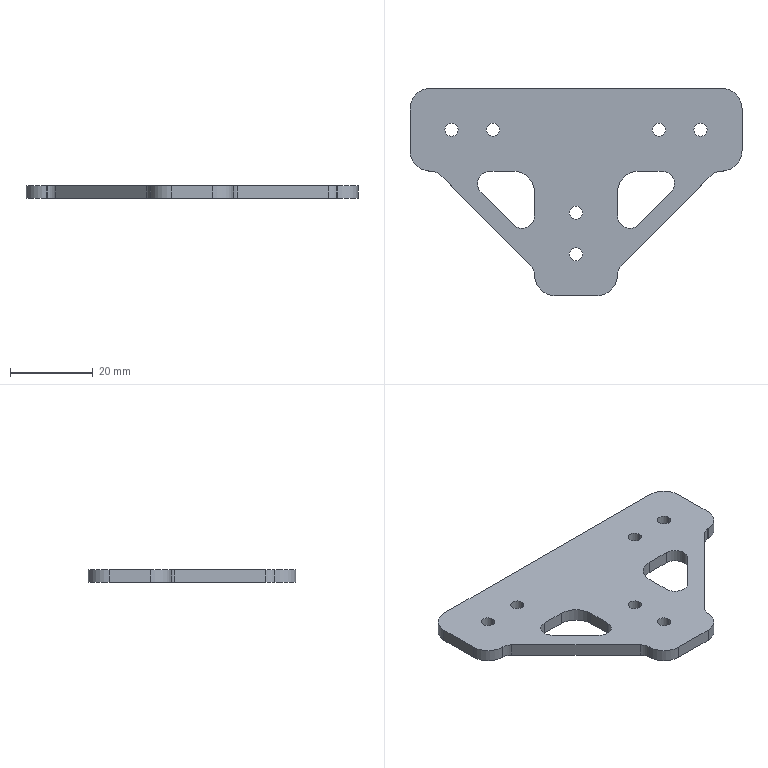Part | SolidWorks | features BaseBody 1 | 1 solid | 47 faces | box 80 x 50 x 3 mm | volume 7234 mm3 | cylinder 29 | plane 18 | commonest cylinder face diameters 3.2 x12 6 x9 10 x8
STEP:
#1=CARTESIAN_POINT('',(28.4,10.,3.));
#2=VERTEX_POINT('',#1);
#3=CARTESIAN_POINT('',(31.6,10.,3.));
#4=VERTEX_POINT('',#3);
#5=CARTESIAN_POINT('',(30.,10.,3.));
#6=DIRECTION('',(0.,0.,1.));
#7=DIRECTION('',(-1.,0.,0.));
#8=AXIS2_PLACEMENT_3D('',#5,#6,#7);
#9=CIRCLE('',#8,1.6);
#10=EDGE_CURVE('',#2,#4,#9,.T.);
#11=ORIENTED_EDGE('',*,*,#10,.T.);
#12=CARTESIAN_POINT('',(31.6,10.,0.));
#13=VERTEX_POINT('',#12);
#14=CARTESIAN_POINT('',(31.6,10.,3.));
#15=DIRECTION('',(0.,0.,-1.));
#16=VECTOR('',#15,1000.);
#17=LINE('',#14,#16);
#18=EDGE_CURVE('',#4,#13,#17,.T.);
#19=ORIENTED_EDGE('',*,*,#18,.T.);
#20=CARTESIAN_POINT('',(28.4,10.,0.));
#21=VERTEX_POINT('',#20);
#22=CARTESIAN_POINT('',(30.,10.,0.));
#23=DIRECTION('',(0.,0.,1.));
#24=DIRECTION('',(-1.,0.,0.));
#25=AXIS2_PLACEMENT_3D('',#22,#23,#24);
#26=CIRCLE('',#25,1.6);
#27=EDGE_CURVE('',#21,#13,#26,.T.);
#28=ORIENTED_EDGE('',*,*,#27,.F.);
#29=CARTESIAN_POINT('',(28.4,10.,3.));
#30=DIRECTION('',(0.,0.,-1.));
#31=VECTOR('',#30,1000.);
#32=LINE('',#29,#31);
#33=EDGE_CURVE('',#2,#21,#32,.T.);
#34=ORIENTED_EDGE('',*,*,#33,.F.);
#35=EDGE_LOOP('',(#11,#19,#28,#34));
#36=FACE_OUTER_BOUND('',#35,.T.);
#37=CARTESIAN_POINT('',(30.,10.,3.));
#38=DIRECTION('',(0.,0.,-1.));
#39=DIRECTION('',(-1.,0.,0.));
#40=AXIS2_PLACEMENT_3D('',#37,#38,#39);
#41=CYLINDRICAL_SURFACE('',#40,1.6);
#42=ADVANCED_FACE('',(#36),#41,.F.);
#43=CARTESIAN_POINT('',(18.4,10.,3.));
#44=VERTEX_POINT('',#43);
#45=CARTESIAN_POINT('',(21.6,10.,3.));
#46=VERTEX_POINT('',#45);
#47=CARTESIAN_POINT('',(20.,10.,3.));
#48=DIRECTION('',(0.,0.,1.));
#49=DIRECTION('',(-1.,0.,0.));
#50=AXIS2_PLACEMENT_3D('',#47,#48,#49);
#51=CIRCLE('',#50,1.6);
#52=EDGE_CURVE('',#44,#46,#51,.T.);
#53=ORIENTED_EDGE('',*,*,#52,.T.);
#54=CARTESIAN_POINT('',(21.6,10.,0.));
#55=VERTEX_POINT('',#54);
#56=CARTESIAN_POINT('',(21.6,10.,3.));
#57=DIRECTION('',(0.,0.,-1.));
#58=VECTOR('',#57,1000.);
#59=LINE('',#56,#58);
#60=EDGE_CURVE('',#46,#55,#59,.T.);
#61=ORIENTED_EDGE('',*,*,#60,.T.);
#62=CARTESIAN_POINT('',(18.4,10.,0.));
#63=VERTEX_POINT('',#62);
#64=CARTESIAN_POINT('',(20.,10.,0.));
#65=DIRECTION('',(0.,0.,1.));
#66=DIRECTION('',(-1.,0.,0.));
#67=AXIS2_PLACEMENT_3D('',#64,#65,#66);
#68=CIRCLE('',#67,1.6);
#69=EDGE_CURVE('',#63,#55,#68,.T.);
#70=ORIENTED_EDGE('',*,*,#69,.F.);
#71=CARTESIAN_POINT('',(18.4,10.,3.));
#72=DIRECTION('',(0.,0.,-1.));
#73=VECTOR('',#72,1000.);
#74=LINE('',#71,#73);
#75=EDGE_CURVE('',#44,#63,#74,.T.);
#76=ORIENTED_EDGE('',*,*,#75,.F.);
#77=EDGE_LOOP('',(#53,#61,#70,#76));
#78=FACE_OUTER_BOUND('',#77,.T.);
#79=CARTESIAN_POINT('',(20.,10.,3.));
#80=DIRECTION('',(0.,0.,-1.));
#81=DIRECTION('',(-1.,0.,0.));
#82=AXIS2_PLACEMENT_3D('',#79,#80,#81);
#83=CYLINDRICAL_SURFACE('',#82,1.6);
#84=ADVANCED_FACE('',(#78),#83,.F.);
#85=CARTESIAN_POINT('',(-1.6,-20.,3.));
#86=VERTEX_POINT('',#85);
#87=CARTESIAN_POINT('',(1.6,-20.,3.));
#88=VERTEX_POINT('',#87);
#89=CARTESIAN_POINT('',(0.,-20.,3.));
#90=DIRECTION('',(0.,0.,1.));
#91=DIRECTION('',(-1.,0.,0.));
#92=AXIS2_PLACEMENT_3D('',#89,#90,#91);
#93=CIRCLE('',#92,1.6);
#94=EDGE_CURVE('',#86,#88,#93,.T.);
#95=ORIENTED_EDGE('',*,*,#94,.T.);
#96=CARTESIAN_POINT('',(1.6,-20.,0.));
#97=VERTEX_POINT('',#96);
#98=CARTESIAN_POINT('',(1.6,-20.,3.));
#99=DIRECTION('',(0.,0.,-1.));
#100=VECTOR('',#99,1000.);
#101=LINE('',#98,#100);
#102=EDGE_CURVE('',#88,#97,#101,.T.);
#103=ORIENTED_EDGE('',*,*,#102,.T.);
#104=CARTESIAN_POINT('',(-1.6,-20.,0.));
#105=VERTEX_POINT('',#104);
#106=CARTESIAN_POINT('',(0.,-20.,0.));
#107=DIRECTION('',(0.,0.,1.));
#108=DIRECTION('',(-1.,0.,0.));
#109=AXIS2_PLACEMENT_3D('',#106,#107,#108);
#110=CIRCLE('',#109,1.6);
#111=EDGE_CURVE('',#105,#97,#110,.T.);
#112=ORIENTED_EDGE('',*,*,#111,.F.);
#113=CARTESIAN_POINT('',(-1.6,-20.,3.));
#114=DIRECTION('',(0.,0.,-1.));
#115=VECTOR('',#114,1000.);
#116=LINE('',#113,#115);
#117=EDGE_CURVE('',#86,#105,#116,.T.);
#118=ORIENTED_EDGE('',*,*,#117,.F.);
#119=EDGE_LOOP('',(#95,#103,#112,#118));
#120=FACE_OUTER_BOUND('',#119,.T.);
#121=CARTESIAN_POINT('',(0.,-20.,3.));
#122=DIRECTION('',(0.,0.,-1.));
#123=DIRECTION('',(-1.,0.,0.));
#124=AXIS2_PLACEMENT_3D('',#121,#122,#123);
#125=CYLINDRICAL_SURFACE('',#124,1.6);
#126=ADVANCED_FACE('',(#120),#125,.F.);
#127=CARTESIAN_POINT('',(-1.6,-10.,3.));
#128=VERTEX_POINT('',#127);
#129=CARTESIAN_POINT('',(1.6,-10.,3.));
#130=VERTEX_POINT('',#129);
#131=CARTESIAN_POINT('',(0.,-10.,3.));
#132=DIRECTION('',(0.,0.,1.));
#133=DIRECTION('',(-1.,0.,0.));
#134=AXIS2_PLACEMENT_3D('',#131,#132,#133);
#135=CIRCLE('',#134,1.6);
#136=EDGE_CURVE('',#128,#130,#135,.T.);
#137=ORIENTED_EDGE('',*,*,#136,.T.);
#138=CARTESIAN_POINT('',(1.6,-10.,0.));
#139=VERTEX_POINT('',#138);
#140=CARTESIAN_POINT('',(1.6,-10.,3.));
#141=DIRECTION('',(0.,0.,-1.));
#142=VECTOR('',#141,1000.);
#143=LINE('',#140,#142);
#144=EDGE_CURVE('',#130,#139,#143,.T.);
#145=ORIENTED_EDGE('',*,*,#144,.T.);
#146=CARTESIAN_POINT('',(-1.6,-10.,0.));
#147=VERTEX_POINT('',#146);
#148=CARTESIAN_POINT('',(0.,-10.,0.));
#149=DIRECTION('',(0.,0.,1.));
#150=DIRECTION('',(-1.,0.,0.));
#151=AXIS2_PLACEMENT_3D('',#148,#149,#150);
#152=CIRCLE('',#151,1.6);
#153=EDGE_CURVE('',#147,#139,#152,.T.);
#154=ORIENTED_EDGE('',*,*,#153,.F.);
#155=CARTESIAN_POINT('',(-1.6,-10.,3.));
#156=DIRECTION('',(0.,0.,-1.));
#157=VECTOR('',#156,1000.);
#158=LINE('',#155,#157);
#159=EDGE_CURVE('',#128,#147,#158,.T.);
#160=ORIENTED_EDGE('',*,*,#159,.F.);
#161=EDGE_LOOP('',(#137,#145,#154,#160));
#162=FACE_OUTER_BOUND('',#161,.T.);
#163=CARTESIAN_POINT('',(0.,-10.,3.));
#164=DIRECTION('',(0.,0.,-1.));
#165=DIRECTION('',(-1.,0.,0.));
#166=AXIS2_PLACEMENT_3D('',#163,#164,#165);
#167=CYLINDRICAL_SURFACE('',#166,1.6);
#168=ADVANCED_FACE('',(#162),#167,.F.);
#169=CARTESIAN_POINT('',(-21.6,10.,3.));
#170=VERTEX_POINT('',#169);
#171=CARTESIAN_POINT('',(-18.4,10.,3.));
#172=VERTEX_POINT('',#171);
#173=CARTESIAN_POINT('',(-20.,10.,3.));
#174=DIRECTION('',(0.,0.,1.));
#175=DIRECTION('',(-1.,0.,0.));
#176=AXIS2_PLACEMENT_3D('',#173,#174,#175);
#177=CIRCLE('',#176,1.6);
#178=EDGE_CURVE('',#170,#172,#177,.T.);
#179=ORIENTED_EDGE('',*,*,#178,.T.);
#180=CARTESIAN_POINT('',(-18.4,10.,0.));
#181=VERTEX_POINT('',#180);
#182=CARTESIAN_POINT('',(-18.4,10.,3.));
#183=DIRECTION('',(0.,0.,-1.));
#184=VECTOR('',#183,1000.);
#185=LINE('',#182,#184);
#186=EDGE_CURVE('',#172,#181,#185,.T.);
#187=ORIENTED_EDGE('',*,*,#186,.T.);
#188=CARTESIAN_POINT('',(-21.6,10.,0.));
#189=VERTEX_POINT('',#188);
#190=CARTESIAN_POINT('',(-20.,10.,0.));
#191=DIRECTION('',(0.,0.,1.));
#192=DIRECTION('',(-1.,0.,0.));
#193=AXIS2_PLACEMENT_3D('',#190,#191,#192);
#194=CIRCLE('',#193,1.6);
#195=EDGE_CURVE('',#189,#181,#194,.T.);
#196=ORIENTED_EDGE('',*,*,#195,.F.);
#197=CARTESIAN_POINT('',(-21.6,10.,3.));
#198=DIRECTION('',(0.,0.,-1.));
#199=VECTOR('',#198,1000.);
#200=LINE('',#197,#199);
#201=EDGE_CURVE('',#170,#189,#200,.T.);
#202=ORIENTED_EDGE('',*,*,#201,.F.);
#203=EDGE_LOOP('',(#179,#187,#196,#202));
#204=FACE_OUTER_BOUND('',#203,.T.);
#205=CARTESIAN_POINT('',(-20.,10.,3.));
#206=DIRECTION('',(0.,0.,-1.));
#207=DIRECTION('',(-1.,0.,0.));
#208=AXIS2_PLACEMENT_3D('',#205,#206,#207);
#209=CYLINDRICAL_SURFACE('',#208,1.6);
#210=ADVANCED_FACE('',(#204),#209,.F.);
#211=CARTESIAN_POINT('',(-31.6,10.,3.));
#212=VERTEX_POINT('',#211);
#213=CARTESIAN_POINT('',(-28.4,10.,3.));
#214=VERTEX_POINT('',#213);
#215=CARTESIAN_POINT('',(-30.,10.,3.));
#216=DIRECTION('',(0.,0.,1.));
#217=DIRECTION('',(-1.,0.,0.));
#218=AXIS2_PLACEMENT_3D('',#215,#216,#217);
#219=CIRCLE('',#218,1.6);
#220=EDGE_CURVE('',#212,#214,#219,.T.);
#221=ORIENTED_EDGE('',*,*,#220,.T.);
#222=CARTESIAN_POINT('',(-28.4,10.,0.));
#223=VERTEX_POINT('',#222);
#224=CARTESIAN_POINT('',(-28.4,10.,3.));
#225=DIRECTION('',(0.,0.,-1.));
#226=VECTOR('',#225,1000.);
#227=LINE('',#224,#226);
#228=EDGE_CURVE('',#214,#223,#227,.T.);
#229=ORIENTED_EDGE('',*,*,#228,.T.);
#230=CARTESIAN_POINT('',(-31.6,10.,0.));
#231=VERTEX_POINT('',#230);
#232=CARTESIAN_POINT('',(-30.,10.,0.));
#233=DIRECTION('',(0.,0.,1.));
#234=DIRECTION('',(-1.,0.,0.));
#235=AXIS2_PLACEMENT_3D('',#232,#233,#234);
#236=CIRCLE('',#235,1.6);
#237=EDGE_CURVE('',#231,#223,#236,.T.);
#238=ORIENTED_EDGE('',*,*,#237,.F.);
#239=CARTESIAN_POINT('',(-31.6,10.,3.));
#240=DIRECTION('',(0.,0.,-1.));
#241=VECTOR('',#240,1000.);
#242=LINE('',#239,#241);
#243=EDGE_CURVE('',#212,#231,#242,.T.);
#244=ORIENTED_EDGE('',*,*,#243,.F.);
#245=EDGE_LOOP('',(#221,#229,#238,#244));
#246=FACE_OUTER_BOUND('',#245,.T.);
#247=CARTESIAN_POINT('',(-30.,10.,3.));
#248=DIRECTION('',(0.,0.,-1.));
#249=DIRECTION('',(-1.,0.,0.));
#250=AXIS2_PLACEMENT_3D('',#247,#248,#249);
#251=CYLINDRICAL_SURFACE('',#250,1.6);
#252=ADVANCED_FACE('',(#246),#251,.F.);
#253=CARTESIAN_POINT('',(-20.757,0.,3.));
#254=VERTEX_POINT('',#253);
#255=CARTESIAN_POINT('',(-23.757,-3.,3.));
#256=VERTEX_POINT('',#255);
#257=CARTESIAN_POINT('',(-20.757,-3.,3.));
#258=DIRECTION('',(0.,0.,1.));
#259=DIRECTION('',(-1.,0.,0.));
#260=AXIS2_PLACEMENT_3D('',#257,#258,#259);
#261=CIRCLE('',#260,3.);
#262=EDGE_CURVE('',#254,#256,#261,.T.);
#263=ORIENTED_EDGE('',*,*,#262,.T.);
#264=CARTESIAN_POINT('',(-23.757,-3.,0.));
#265=VERTEX_POINT('',#264);
#266=CARTESIAN_POINT('',(-23.757,-3.,3.));
#267=DIRECTION('',(0.,0.,-1.));
#268=VECTOR('',#267,1000.);
#269=LINE('',#266,#268);
#270=EDGE_CURVE('',#256,#265,#269,.T.);
#271=ORIENTED_EDGE('',*,*,#270,.T.);
#272=CARTESIAN_POINT('',(-20.757,0.,0.));
#273=VERTEX_POINT('',#272);
#274=CARTESIAN_POINT('',(-20.757,-3.,0.));
#275=DIRECTION('',(0.,0.,1.));
#276=DIRECTION('',(-1.,0.,0.));
#277=AXIS2_PLACEMENT_3D('',#274,#275,#276);
#278=CIRCLE('',#277,3.);
#279=EDGE_CURVE('',#273,#265,#278,.T.);
#280=ORIENTED_EDGE('',*,*,#279,.F.);
#281=CARTESIAN_POINT('',(-20.757,0.,3.));
#282=DIRECTION('',(0.,0.,-1.));
#283=VECTOR('',#282,1000.);
#284=LINE('',#281,#283);
#285=EDGE_CURVE('',#254,#273,#284,.T.);
#286=ORIENTED_EDGE('',*,*,#285,.F.);
#287=EDGE_LOOP('',(#263,#271,#280,#286));
#288=FACE_OUTER_BOUND('',#287,.T.);
#289=CARTESIAN_POINT('',(-20.757,-3.,3.));
#290=DIRECTION('',(0.,0.,-1.));
#291=DIRECTION('',(-1.,0.,0.));
#292=AXIS2_PLACEMENT_3D('',#289,#290,#291);
#293=CYLINDRICAL_SURFACE('',#292,3.);
#294=ADVANCED_FACE('',(#288),#293,.F.);
#295=ORIENTED_EDGE('',*,*,#10,.F.);
#296=CARTESIAN_POINT('',(30.,10.,3.));
#297=DIRECTION('',(0.,0.,1.));
#298=DIRECTION('',(-1.,0.,0.));
#299=AXIS2_PLACEMENT_3D('',#296,#297,#298);
#300=CIRCLE('',#299,1.6);
#301=EDGE_CURVE('',#4,#2,#300,.T.);
#302=ORIENTED_EDGE('',*,*,#301,.F.);
#303=EDGE_LOOP('',(#295,#302));
#304=FACE_BOUND('',#303,.T.);
#305=ORIENTED_EDGE('',*,*,#52,.F.);
#306=CARTESIAN_POINT('',(20.,10.,3.));
#307=DIRECTION('',(0.,0.,1.));
#308=DIRECTION('',(-1.,0.,0.));
#309=AXIS2_PLACEMENT_3D('',#306,#307,#308);
#310=CIRCLE('',#309,1.6);
#311=EDGE_CURVE('',#46,#44,#310,.T.);
#312=ORIENTED_EDGE('',*,*,#311,.F.);
#313=EDGE_LOOP('',(#305,#312));
#314=FACE_BOUND('',#313,.T.);
#315=ORIENTED_EDGE('',*,*,#94,.F.);
#316=CARTESIAN_POINT('',(0.,-20.,3.));
#317=DIRECTION('',(0.,0.,1.));
#318=DIRECTION('',(-1.,0.,0.));
#319=AXIS2_PLACEMENT_3D('',#316,#317,#318);
#320=CIRCLE('',#319,1.6);
#321=EDGE_CURVE('',#88,#86,#320,.T.);
#322=ORIENTED_EDGE('',*,*,#321,.F.);
#323=EDGE_LOOP('',(#315,#322));
#324=FACE_BOUND('',#323,.T.);
#325=ORIENTED_EDGE('',*,*,#136,.F.);
#326=CARTESIAN_POINT('',(0.,-10.,3.));
#327=DIRECTION('',(0.,0.,1.));
#328=DIRECTION('',(-1.,0.,0.));
#329=AXIS2_PLACEMENT_3D('',#326,#327,#328);
#330=CIRCLE('',#329,1.6);
#331=EDGE_CURVE('',#130,#128,#330,.T.);
#332=ORIENTED_EDGE('',*,*,#331,.F.);
#333=EDGE_LOOP('',(#325,#332));
#334=FACE_BOUND('',#333,.T.);
#335=ORIENTED_EDGE('',*,*,#178,.F.);
#336=CARTESIAN_POINT('',(-20.,10.,3.));
#337=DIRECTION('',(0.,0.,1.));
#338=DIRECTION('',(-1.,0.,0.));
#339=AXIS2_PLACEMENT_3D('',#336,#337,#338);
#340=CIRCLE('',#339,1.6);
#341=EDGE_CURVE('',#172,#170,#340,.T.);
#342=ORIENTED_EDGE('',*,*,#341,.F.);
#343=EDGE_LOOP('',(#335,#342));
#344=FACE_BOUND('',#343,.T.);
#345=ORIENTED_EDGE('',*,*,#220,.F.);
#346=CARTESIAN_POINT('',(-30.,10.,3.));
#347=DIRECTION('',(0.,0.,1.));
#348=DIRECTION('',(-1.,0.,0.));
#349=AXIS2_PLACEMENT_3D('',#346,#347,#348);
#350=CIRCLE('',#349,1.6);
#351=EDGE_CURVE('',#214,#212,#350,.T.);
#352=ORIENTED_EDGE('',*,*,#351,.F.);
#353=EDGE_LOOP('',(#345,#352));
#354=FACE_BOUND('',#353,.T.);
#355=CARTESIAN_POINT('',(-32.778,-0.8787,3.));
#356=VERTEX_POINT('',#355);
#357=CARTESIAN_POINT('',(-34.899,0.,3.));
#358=VERTEX_POINT('',#357);
#359=CARTESIAN_POINT('',(-34.899,-3.,3.));
#360=DIRECTION('',(0.,0.,1.));
#361=DIRECTION('',(-1.,0.,0.));
#362=AXIS2_PLACEMENT_3D('',#359,#360,#361);
#363=CIRCLE('',#362,3.);
#364=EDGE_CURVE('',#356,#358,#363,.T.);
#365=ORIENTED_EDGE('',*,*,#364,.F.);
#366=CARTESIAN_POINT('',(-10.879,-22.778,3.));
#367=VERTEX_POINT('',#366);
#368=CARTESIAN_POINT('',(-10.879,-22.778,3.));
#369=DIRECTION('',(-0.7071,0.7071,0.));
#370=VECTOR('',#369,1000.);
#371=LINE('',#368,#370);
#372=EDGE_CURVE('',#367,#356,#371,.T.);
#373=ORIENTED_EDGE('',*,*,#372,.F.);
#374=CARTESIAN_POINT('',(-10.,-24.899,3.));
#375=VERTEX_POINT('',#374);
#376=CARTESIAN_POINT('',(-13.,-24.899,3.));
#377=DIRECTION('',(0.,0.,1.));
#378=DIRECTION('',(-1.,0.,0.));
#379=AXIS2_PLACEMENT_3D('',#376,#377,#378);
#380=CIRCLE('',#379,3.);
#381=EDGE_CURVE('',#375,#367,#380,.T.);
#382=ORIENTED_EDGE('',*,*,#381,.F.);
#383=CARTESIAN_POINT('',(-10.,-25.,3.));
#384=VERTEX_POINT('',#383);
#385=CARTESIAN_POINT('',(-10.,-30.,3.));
#386=DIRECTION('',(0.,-1.,0.));
#387=VECTOR('',#386,1000.);
#388=LINE('',#385,#387);
#389=EDGE_CURVE('',#375,#384,#388,.T.);
#390=ORIENTED_EDGE('',*,*,#389,.T.);
#391=CARTESIAN_POINT('',(-5.,-30.,3.));
#392=VERTEX_POINT('',#391);
#393=CARTESIAN_POINT('',(-5.,-25.,3.));
#394=DIRECTION('',(0.,0.,-1.));
#395=DIRECTION('',(-1.,0.,0.));
#396=AXIS2_PLACEMENT_3D('',#393,#394,#395);
#397=CIRCLE('',#396,5.);
#398=EDGE_CURVE('',#392,#384,#397,.T.);
#399=ORIENTED_EDGE('',*,*,#398,.F.);
#400=CARTESIAN_POINT('',(5.,-30.,3.));
#401=VERTEX_POINT('',#400);
#402=CARTESIAN_POINT('',(0.,-30.,3.));
#403=DIRECTION('',(-1.,0.,0.));
#404=VECTOR('',#403,1000.);
#405=LINE('',#402,#404);
#406=EDGE_CURVE('',#401,#392,#405,.T.);
#407=ORIENTED_EDGE('',*,*,#406,.F.);
#408=CARTESIAN_POINT('',(10.,-25.,3.));
#409=VERTEX_POINT('',#408);
#410=CARTESIAN_POINT('',(5.,-25.,3.));
#411=DIRECTION('',(0.,0.,-1.));
#412=DIRECTION('',(-1.,0.,0.));
#413=AXIS2_PLACEMENT_3D('',#410,#411,#412);
#414=CIRCLE('',#413,5.);
#415=EDGE_CURVE('',#409,#401,#414,.T.);
#416=ORIENTED_EDGE('',*,*,#415,.F.);
#417=CARTESIAN_POINT('',(10.,-24.899,3.));
#418=VERTEX_POINT('',#417);
#419=CARTESIAN_POINT('',(10.,0.,3.));
#420=DIRECTION('',(0.,1.,0.));
#421=VECTOR('',#420,1000.);
#422=LINE('',#419,#421);
#423=EDGE_CURVE('',#409,#418,#422,.T.);
#424=ORIENTED_EDGE('',*,*,#423,.T.);
#425=CARTESIAN_POINT('',(10.879,-22.778,3.));
#426=VERTEX_POINT('',#425);
#427=CARTESIAN_POINT('',(13.,-24.899,3.));
#428=DIRECTION('',(0.,0.,1.));
#429=DIRECTION('',(-1.,0.,0.));
#430=AXIS2_PLACEMENT_3D('',#427,#428,#429);
#431=CIRCLE('',#430,3.);
#432=EDGE_CURVE('',#426,#418,#431,.T.);
#433=ORIENTED_EDGE('',*,*,#432,.F.);
#434=CARTESIAN_POINT('',(32.778,-0.8787,3.));
#435=VERTEX_POINT('',#434);
#436=CARTESIAN_POINT('',(32.778,-0.8787,3.));
#437=DIRECTION('',(-0.7071,-0.7071,0.));
#438=VECTOR('',#437,1000.);
#439=LINE('',#436,#438);
#440=EDGE_CURVE('',#435,#426,#439,.T.);
#441=ORIENTED_EDGE('',*,*,#440,.F.);
#442=CARTESIAN_POINT('',(34.899,0.,3.));
#443=VERTEX_POINT('',#442);
#444=CARTESIAN_POINT('',(34.899,-3.,3.));
#445=DIRECTION('',(0.,0.,1.));
#446=DIRECTION('',(-1.,0.,0.));
#447=AXIS2_PLACEMENT_3D('',#444,#445,#446);
#448=CIRCLE('',#447,3.);
#449=EDGE_CURVE('',#443,#435,#448,.T.);
#450=ORIENTED_EDGE('',*,*,#449,.F.);
#451=CARTESIAN_POINT('',(35.,0.,3.));
#452=VERTEX_POINT('',#451);
#453=CARTESIAN_POINT('',(40.,0.,3.));
#454=DIRECTION('',(1.,0.,0.));
#455=VECTOR('',#454,1000.);
#456=LINE('',#453,#455);
#457=EDGE_CURVE('',#443,#452,#456,.T.);
#458=ORIENTED_EDGE('',*,*,#457,.T.);
#459=CARTESIAN_POINT('',(40.,5.,3.));
#460=VERTEX_POINT('',#459);
#461=CARTESIAN_POINT('',(35.,5.,3.));
#462=DIRECTION('',(0.,0.,-1.));
#463=DIRECTION('',(-1.,0.,0.));
#464=AXIS2_PLACEMENT_3D('',#461,#462,#463);
#465=CIRCLE('',#464,5.);
#466=EDGE_CURVE('',#460,#452,#465,.T.);
#467=ORIENTED_EDGE('',*,*,#466,.F.);
#468=CARTESIAN_POINT('',(40.,15.,3.));
#469=VERTEX_POINT('',#468);
#470=CARTESIAN_POINT('',(40.,0.,3.));
#471=DIRECTION('',(0.,-1.,0.));
#472=VECTOR('',#471,1000.);
#473=LINE('',#470,#472);
#474=EDGE_CURVE('',#469,#460,#473,.T.);
#475=ORIENTED_EDGE('',*,*,#474,.F.);
#476=CARTESIAN_POINT('',(35.,20.,3.));
#477=VERTEX_POINT('',#476);
#478=CARTESIAN_POINT('',(35.,15.,3.));
#479=DIRECTION('',(0.,0.,-1.));
#480=DIRECTION('',(-1.,0.,0.));
#481=AXIS2_PLACEMENT_3D('',#478,#479,#480);
#482=CIRCLE('',#481,5.);
#483=EDGE_CURVE('',#477,#469,#482,.T.);
#484=ORIENTED_EDGE('',*,*,#483,.F.);
#485=CARTESIAN_POINT('',(-35.,20.,3.));
#486=VERTEX_POINT('',#485);
#487=CARTESIAN_POINT('',(0.,20.,3.));
#488=DIRECTION('',(1.,0.,0.));
#489=VECTOR('',#488,1000.);
#490=LINE('',#487,#489);
#491=EDGE_CURVE('',#486,#477,#490,.T.);
#492=ORIENTED_EDGE('',*,*,#491,.F.);
#493=CARTESIAN_POINT('',(-40.,15.,3.));
#494=VERTEX_POINT('',#493);
#495=CARTESIAN_POINT('',(-35.,15.,3.));
#496=DIRECTION('',(0.,0.,-1.));
#497=DIRECTION('',(-1.,0.,0.));
#498=AXIS2_PLACEMENT_3D('',#495,#496,#497);
#499=CIRCLE('',#498,5.);
#500=EDGE_CURVE('',#494,#486,#499,.T.);
#501=ORIENTED_EDGE('',*,*,#500,.F.);
#502=CARTESIAN_POINT('',(-40.,5.,3.));
#503=VERTEX_POINT('',#502);
#504=CARTESIAN_POINT('',(-40.,0.,3.));
#505=DIRECTION('',(0.,1.,0.));
#506=VECTOR('',#505,1000.);
#507=LINE('',#504,#506);
#508=EDGE_CURVE('',#503,#494,#507,.T.);
#509=ORIENTED_EDGE('',*,*,#508,.F.);
#510=CARTESIAN_POINT('',(-35.,0.,3.));
#511=VERTEX_POINT('',#510);
#512=CARTESIAN_POINT('',(-35.,5.,3.));
#513=DIRECTION('',(0.,0.,-1.));
#514=DIRECTION('',(-1.,0.,0.));
#515=AXIS2_PLACEMENT_3D('',#512,#513,#514);
#516=CIRCLE('',#515,5.);
#517=EDGE_CURVE('',#511,#503,#516,.T.);
#518=ORIENTED_EDGE('',*,*,#517,.F.);
#519=CARTESIAN_POINT('',(-10.,0.,3.));
#520=DIRECTION('',(1.,0.,0.));
#521=VECTOR('',#520,1000.);
#522=LINE('',#519,#521);
#523=EDGE_CURVE('',#511,#358,#522,.T.);
#524=ORIENTED_EDGE('',*,*,#523,.T.);
#525=EDGE_LOOP('',(#365,#373,#382,#390,#399,#407,#416,#424,#433,#441,#450,#458,#467,#475,#484,#492,#501,#509,#518,#524));
#526=FACE_OUTER_BOUND('',#525,.T.);
#527=CARTESIAN_POINT('',(10.,-10.757,3.));
#528=VERTEX_POINT('',#527);
#529=CARTESIAN_POINT('',(15.121,-12.879,3.));
#530=VERTEX_POINT('',#529);
#531=CARTESIAN_POINT('',(13.,-10.757,3.));
#532=DIRECTION('',(0.,0.,1.));
#533=DIRECTION('',(-1.,0.,0.));
#534=AXIS2_PLACEMENT_3D('',#531,#532,#533);
#535=CIRCLE('',#534,3.);
#536=EDGE_CURVE('',#528,#530,#535,.T.);
#537=ORIENTED_EDGE('',*,*,#536,.F.);
#538=CARTESIAN_POINT('',(10.,-5.,3.));
#539=VERTEX_POINT('',#538);
#540=CARTESIAN_POINT('',(10.,0.,3.));
#541=DIRECTION('',(0.,-1.,0.));
#542=VECTOR('',#541,1000.);
#543=LINE('',#540,#542);
#544=EDGE_CURVE('',#539,#528,#543,.T.);
#545=ORIENTED_EDGE('',*,*,#544,.F.);
#546=CARTESIAN_POINT('',(15.,0.,3.));
#547=VERTEX_POINT('',#546);
#548=CARTESIAN_POINT('',(15.,-5.,3.));
#549=DIRECTION('',(0.,0.,1.));
#550=DIRECTION('',(1.,0.,0.));
#551=AXIS2_PLACEMENT_3D('',#548,#549,#550);
#552=CIRCLE('',#551,5.);
#553=EDGE_CURVE('',#547,#539,#552,.T.);
#554=ORIENTED_EDGE('',*,*,#553,.F.);
#555=CARTESIAN_POINT('',(20.757,0.,3.));
#556=VERTEX_POINT('',#555);
#557=CARTESIAN_POINT('',(0.,0.,3.));
#558=DIRECTION('',(-1.,0.,0.));
#559=VECTOR('',#558,1000.);
#560=LINE('',#557,#559);
#561=EDGE_CURVE('',#556,#547,#560,.T.);
#562=ORIENTED_EDGE('',*,*,#561,.F.);
#563=CARTESIAN_POINT('',(22.879,-5.121,3.));
#564=VERTEX_POINT('',#563);
#565=CARTESIAN_POINT('',(20.757,-3.,3.));
#566=DIRECTION('',(0.,0.,1.));
#567=DIRECTION('',(-1.,0.,0.));
#568=AXIS2_PLACEMENT_3D('',#565,#566,#567);
#569=CIRCLE('',#568,3.);
#570=EDGE_CURVE('',#564,#556,#569,.T.);
#571=ORIENTED_EDGE('',*,*,#570,.F.);
#572=CARTESIAN_POINT('',(15.121,-12.879,3.));
#573=DIRECTION('',(0.7071,0.7071,0.));
#574=VECTOR('',#573,1000.);
#575=LINE('',#572,#574);
#576=EDGE_CURVE('',#530,#564,#575,.T.);
#577=ORIENTED_EDGE('',*,*,#576,.F.);
#578=EDGE_LOOP('',(#537,#545,#554,#562,#571,#577));
#579=FACE_BOUND('',#578,.T.);
#580=CARTESIAN_POINT('',(-22.879,-5.121,3.));
#581=VERTEX_POINT('',#580);
#582=CARTESIAN_POINT('',(-15.121,-12.879,3.));
#583=VERTEX_POINT('',#582);
#584=CARTESIAN_POINT('',(-22.879,-5.121,3.));
#585=DIRECTION('',(0.7071,-0.7071,0.));
#586=VECTOR('',#585,1000.);
#587=LINE('',#584,#586);
#588=EDGE_CURVE('',#581,#583,#587,.T.);
#589=ORIENTED_EDGE('',*,*,#588,.F.);
#590=CARTESIAN_POINT('',(-20.757,-3.,3.));
#591=DIRECTION('',(0.,0.,1.));
#592=DIRECTION('',(-1.,0.,0.));
#593=AXIS2_PLACEMENT_3D('',#590,#591,#592);
#594=CIRCLE('',#593,3.);
#595=EDGE_CURVE('',#256,#581,#594,.T.);
#596=ORIENTED_EDGE('',*,*,#595,.F.);
#597=ORIENTED_EDGE('',*,*,#262,.F.);
#598=CARTESIAN_POINT('',(-15.,0.,3.));
#599=VERTEX_POINT('',#598);
#600=CARTESIAN_POINT('',(0.,0.,3.));
#601=DIRECTION('',(-1.,0.,0.));
#602=VECTOR('',#601,1000.);
#603=LINE('',#600,#602);
#604=EDGE_CURVE('',#599,#254,#603,.T.);
#605=ORIENTED_EDGE('',*,*,#604,.F.);
#606=CARTESIAN_POINT('',(-10.,-5.,3.));
#607=VERTEX_POINT('',#606);
#608=CARTESIAN_POINT('',(-15.,-5.,3.));
#609=DIRECTION('',(0.,0.,1.));
#610=DIRECTION('',(1.,0.,0.));
#611=AXIS2_PLACEMENT_3D('',#608,#609,#610);
#612=CIRCLE('',#611,5.);
#613=EDGE_CURVE('',#607,#599,#612,.T.);
#614=ORIENTED_EDGE('',*,*,#613,.F.);
#615=CARTESIAN_POINT('',(-10.,-10.757,3.));
#616=VERTEX_POINT('',#615);
#617=CARTESIAN_POINT('',(-10.,0.,3.));
#618=DIRECTION('',(0.,1.,0.));
#619=VECTOR('',#618,1000.);
#620=LINE('',#617,#619);
#621=EDGE_CURVE('',#616,#607,#620,.T.);
#622=ORIENTED_EDGE('',*,*,#621,.F.);
#623=CARTESIAN_POINT('',(-13.,-10.757,3.));
#624=DIRECTION('',(0.,0.,1.));
#625=DIRECTION('',(-1.,0.,0.));
#626=AXIS2_PLACEMENT_3D('',#623,#624,#625);
#627=CIRCLE('',#626,3.);
#628=EDGE_CURVE('',#583,#616,#627,.T.);
#629=ORIENTED_EDGE('',*,*,#628,.F.);
#630=EDGE_LOOP('',(#589,#596,#597,#605,#614,#622,#629));
#631=FACE_BOUND('',#630,.T.);
#632=CARTESIAN_POINT('',(0.,0.,3.));
#633=DIRECTION('',(0.,0.,-1.));
#634=DIRECTION('',(-1.,0.,0.));
#635=AXIS2_PLACEMENT_3D('',#632,#633,#634);
#636=PLANE('',#635);
#637=ADVANCED_FACE('',(#304,#314,#324,#334,#344,#354,#526,#579,#631),#636,.F.);
#638=ORIENTED_EDGE('',*,*,#18,.F.);
#639=ORIENTED_EDGE('',*,*,#301,.T.);
#640=ORIENTED_EDGE('',*,*,#33,.T.);
#641=CARTESIAN_POINT('',(30.,10.,0.));
#642=DIRECTION('',(0.,0.,1.));
#643=DIRECTION('',(-1.,0.,0.));
#644=AXIS2_PLACEMENT_3D('',#641,#642,#643);
#645=CIRCLE('',#644,1.6);
#646=EDGE_CURVE('',#13,#21,#645,.T.);
#647=ORIENTED_EDGE('',*,*,#646,.F.);
#648=EDGE_LOOP('',(#638,#639,#640,#647));
#649=FACE_OUTER_BOUND('',#648,.T.);
#650=CARTESIAN_POINT('',(30.,10.,3.));
#651=DIRECTION('',(0.,0.,-1.));
#652=DIRECTION('',(-1.,0.,0.));
#653=AXIS2_PLACEMENT_3D('',#650,#651,#652);
#654=CYLINDRICAL_SURFACE('',#653,1.6);
#655=ADVANCED_FACE('',(#649),#654,.F.);
#656=ORIENTED_EDGE('',*,*,#60,.F.);
#657=ORIENTED_EDGE('',*,*,#311,.T.);
#658=ORIENTED_EDGE('',*,*,#75,.T.);
#659=CARTESIAN_POINT('',(20.,10.,0.));
#660=DIRECTION('',(0.,0.,1.));
#661=DIRECTION('',(-1.,0.,0.));
#662=AXIS2_PLACEMENT_3D('',#659,#660,#661);
#663=CIRCLE('',#662,1.6);
#664=EDGE_CURVE('',#55,#63,#663,.T.);
#665=ORIENTED_EDGE('',*,*,#664,.F.);
#666=EDGE_LOOP('',(#656,#657,#658,#665));
#667=FACE_OUTER_BOUND('',#666,.T.);
#668=CARTESIAN_POINT('',(20.,10.,3.));
#669=DIRECTION('',(0.,0.,-1.));
#670=DIRECTION('',(-1.,0.,0.));
#671=AXIS2_PLACEMENT_3D('',#668,#669,#670);
#672=CYLINDRICAL_SURFACE('',#671,1.6);
#673=ADVANCED_FACE('',(#667),#672,.F.);
#674=ORIENTED_EDGE('',*,*,#102,.F.);
#675=ORIENTED_EDGE('',*,*,#321,.T.);
#676=ORIENTED_EDGE('',*,*,#117,.T.);
#677=CARTESIAN_POINT('',(0.,-20.,0.));
#678=DIRECTION('',(0.,0.,1.));
#679=DIRECTION('',(-1.,0.,0.));
#680=AXIS2_PLACEMENT_3D('',#677,#678,#679);
#681=CIRCLE('',#680,1.6);
#682=EDGE_CURVE('',#97,#105,#681,.T.);
#683=ORIENTED_EDGE('',*,*,#682,.F.);
#684=EDGE_LOOP('',(#674,#675,#676,#683));
#685=FACE_OUTER_BOUND('',#684,.T.);
#686=CARTESIAN_POINT('',(0.,-20.,3.));
#687=DIRECTION('',(0.,0.,-1.));
#688=DIRECTION('',(-1.,0.,0.));
#689=AXIS2_PLACEMENT_3D('',#686,#687,#688);
#690=CYLINDRICAL_SURFACE('',#689,1.6);
#691=ADVANCED_FACE('',(#685),#690,.F.);
#692=ORIENTED_EDGE('',*,*,#144,.F.);
#693=ORIENTED_EDGE('',*,*,#331,.T.);
#694=ORIENTED_EDGE('',*,*,#159,.T.);
#695=CARTESIAN_POINT('',(0.,-10.,0.));
#696=DIRECTION('',(0.,0.,1.));
#697=DIRECTION('',(-1.,0.,0.));
#698=AXIS2_PLACEMENT_3D('',#695,#696,#697);
#699=CIRCLE('',#698,1.6);
#700=EDGE_CURVE('',#139,#147,#699,.T.);
#701=ORIENTED_EDGE('',*,*,#700,.F.);
#702=EDGE_LOOP('',(#692,#693,#694,#701));
#703=FACE_OUTER_BOUND('',#702,.T.);
#704=CARTESIAN_POINT('',(0.,-10.,3.));
#705=DIRECTION('',(0.,0.,-1.));
#706=DIRECTION('',(-1.,0.,0.));
#707=AXIS2_PLACEMENT_3D('',#704,#705,#706);
#708=CYLINDRICAL_SURFACE('',#707,1.6);
#709=ADVANCED_FACE('',(#703),#708,.F.);
#710=ORIENTED_EDGE('',*,*,#186,.F.);
#711=ORIENTED_EDGE('',*,*,#341,.T.);
#712=ORIENTED_EDGE('',*,*,#201,.T.);
#713=CARTESIAN_POINT('',(-20.,10.,0.));
#714=DIRECTION('',(0.,0.,1.));
#715=DIRECTION('',(-1.,0.,0.));
#716=AXIS2_PLACEMENT_3D('',#713,#714,#715);
#717=CIRCLE('',#716,1.6);
#718=EDGE_CURVE('',#181,#189,#717,.T.);
#719=ORIENTED_EDGE('',*,*,#718,.F.);
#720=EDGE_LOOP('',(#710,#711,#712,#719));
#721=FACE_OUTER_BOUND('',#720,.T.);
#722=CARTESIAN_POINT('',(-20.,10.,3.));
#723=DIRECTION('',(0.,0.,-1.));
#724=DIRECTION('',(-1.,0.,0.));
#725=AXIS2_PLACEMENT_3D('',#722,#723,#724);
#726=CYLINDRICAL_SURFACE('',#725,1.6);
#727=ADVANCED_FACE('',(#721),#726,.F.);
#728=ORIENTED_EDGE('',*,*,#228,.F.);
#729=ORIENTED_EDGE('',*,*,#351,.T.);
#730=ORIENTED_EDGE('',*,*,#243,.T.);
#731=CARTESIAN_POINT('',(-30.,10.,0.));
#732=DIRECTION('',(0.,0.,1.));
#733=DIRECTION('',(-1.,0.,0.));
#734=AXIS2_PLACEMENT_3D('',#731,#732,#733);
#735=CIRCLE('',#734,1.6);
#736=EDGE_CURVE('',#223,#231,#735,.T.);
#737=ORIENTED_EDGE('',*,*,#736,.F.);
#738=EDGE_LOOP('',(#728,#729,#730,#737));
#739=FACE_OUTER_BOUND('',#738,.T.);
#740=CARTESIAN_POINT('',(-30.,10.,3.));
#741=DIRECTION('',(0.,0.,-1.));
#742=DIRECTION('',(-1.,0.,0.));
#743=AXIS2_PLACEMENT_3D('',#740,#741,#742);
#744=CYLINDRICAL_SURFACE('',#743,1.6);
#745=ADVANCED_FACE('',(#739),#744,.F.);
#746=CARTESIAN_POINT('',(-34.899,0.,0.));
#747=VERTEX_POINT('',#746);
#748=CARTESIAN_POINT('',(-34.899,0.,3.));
#749=DIRECTION('',(0.,0.,1.));
#750=VECTOR('',#749,1000.);
#751=LINE('',#748,#750);
#752=EDGE_CURVE('',#747,#358,#751,.T.);
#753=ORIENTED_EDGE('',*,*,#752,.F.);
#754=CARTESIAN_POINT('',(-32.778,-0.8787,0.));
#755=VERTEX_POINT('',#754);
#756=CARTESIAN_POINT('',(-34.899,-3.,0.));
#757=DIRECTION('',(0.,0.,1.));
#758=DIRECTION('',(-1.,0.,0.));
#759=AXIS2_PLACEMENT_3D('',#756,#757,#758);
#760=CIRCLE('',#759,3.);
#761=EDGE_CURVE('',#755,#747,#760,.T.);
#762=ORIENTED_EDGE('',*,*,#761,.F.);
#763=CARTESIAN_POINT('',(-32.778,-0.8787,3.));
#764=DIRECTION('',(0.,0.,-1.));
#765=VECTOR('',#764,1000.);
#766=LINE('',#763,#765);
#767=EDGE_CURVE('',#356,#755,#766,.T.);
#768=ORIENTED_EDGE('',*,*,#767,.F.);
#769=ORIENTED_EDGE('',*,*,#364,.T.);
#770=EDGE_LOOP('',(#753,#762,#768,#769));
#771=FACE_OUTER_BOUND('',#770,.T.);
#772=CARTESIAN_POINT('',(-34.899,-3.,3.));
#773=DIRECTION('',(0.,0.,-1.));
#774=DIRECTION('',(-1.,0.,0.));
#775=AXIS2_PLACEMENT_3D('',#772,#773,#774);
#776=CYLINDRICAL_SURFACE('',#775,3.);
#777=ADVANCED_FACE('',(#771),#776,.F.);
#778=ORIENTED_EDGE('',*,*,#372,.T.);
#779=ORIENTED_EDGE('',*,*,#767,.T.);
#780=CARTESIAN_POINT('',(-10.879,-22.778,0.));
#781=VERTEX_POINT('',#780);
#782=CARTESIAN_POINT('',(-33.657,0.,0.));
#783=DIRECTION('',(0.7071,-0.7071,0.));
#784=VECTOR('',#783,1000.);
#785=LINE('',#782,#784);
#786=EDGE_CURVE('',#755,#781,#785,.T.);
#787=ORIENTED_EDGE('',*,*,#786,.T.);
#788=CARTESIAN_POINT('',(-10.879,-22.778,3.));
#789=DIRECTION('',(0.,0.,1.));
#790=VECTOR('',#789,1000.);
#791=LINE('',#788,#790);
#792=EDGE_CURVE('',#781,#367,#791,.T.);
#793=ORIENTED_EDGE('',*,*,#792,.T.);
#794=EDGE_LOOP('',(#778,#779,#787,#793));
#795=FACE_OUTER_BOUND('',#794,.T.);
#796=CARTESIAN_POINT('',(-33.657,0.,3.));
#797=DIRECTION('',(-0.7071,-0.7071,0.));
#798=DIRECTION('',(0.7071,-0.7071,0.));
#799=AXIS2_PLACEMENT_3D('',#796,#797,#798);
#800=PLANE('',#799);
#801=ADVANCED_FACE('',(#795),#800,.T.);
#802=ORIENTED_EDGE('',*,*,#792,.F.);
#803=CARTESIAN_POINT('',(-10.,-24.899,0.));
#804=VERTEX_POINT('',#803);
#805=CARTESIAN_POINT('',(-13.,-24.899,0.));
#806=DIRECTION('',(0.,0.,1.));
#807=DIRECTION('',(-1.,0.,0.));
#808=AXIS2_PLACEMENT_3D('',#805,#806,#807);
#809=CIRCLE('',#808,3.);
#810=EDGE_CURVE('',#804,#781,#809,.T.);
#811=ORIENTED_EDGE('',*,*,#810,.F.);
#812=CARTESIAN_POINT('',(-10.,-24.899,3.));
#813=DIRECTION('',(0.,0.,-1.));
#814=VECTOR('',#813,1000.);
#815=LINE('',#812,#814);
#816=EDGE_CURVE('',#375,#804,#815,.T.);
#817=ORIENTED_EDGE('',*,*,#816,.F.);
#818=ORIENTED_EDGE('',*,*,#381,.T.);
#819=EDGE_LOOP('',(#802,#811,#817,#818));
#820=FACE_OUTER_BOUND('',#819,.T.);
#821=CARTESIAN_POINT('',(-13.,-24.899,3.));
#822=DIRECTION('',(0.,0.,-1.));
#823=DIRECTION('',(-1.,0.,0.));
#824=AXIS2_PLACEMENT_3D('',#821,#822,#823);
#825=CYLINDRICAL_SURFACE('',#824,3.);
#826=ADVANCED_FACE('',(#820),#825,.F.);
#827=CARTESIAN_POINT('',(-10.,-25.,0.));
#828=VERTEX_POINT('',#827);
#829=CARTESIAN_POINT('',(-5.,-30.,0.));
#830=VERTEX_POINT('',#829);
#831=CARTESIAN_POINT('',(-5.,-25.,0.));
#832=DIRECTION('',(0.,0.,1.));
#833=DIRECTION('',(-1.,0.,0.));
#834=AXIS2_PLACEMENT_3D('',#831,#832,#833);
#835=CIRCLE('',#834,5.);
#836=EDGE_CURVE('',#828,#830,#835,.T.);
#837=ORIENTED_EDGE('',*,*,#836,.T.);
#838=CARTESIAN_POINT('',(-5.,-30.,3.));
#839=DIRECTION('',(0.,0.,1.));
#840=VECTOR('',#839,1000.);
#841=LINE('',#838,#840);
#842=EDGE_CURVE('',#830,#392,#841,.T.);
#843=ORIENTED_EDGE('',*,*,#842,.T.);
#844=ORIENTED_EDGE('',*,*,#398,.T.);
#845=CARTESIAN_POINT('',(-10.,-25.,3.));
#846=DIRECTION('',(0.,0.,-1.));
#847=VECTOR('',#846,1000.);
#848=LINE('',#845,#847);
#849=EDGE_CURVE('',#384,#828,#848,.T.);
#850=ORIENTED_EDGE('',*,*,#849,.T.);
#851=EDGE_LOOP('',(#837,#843,#844,#850));
#852=FACE_OUTER_BOUND('',#851,.T.);
#853=CARTESIAN_POINT('',(-5.,-25.,3.));
#854=DIRECTION('',(0.,0.,-1.));
#855=DIRECTION('',(-1.,0.,0.));
#856=AXIS2_PLACEMENT_3D('',#853,#854,#855);
#857=CYLINDRICAL_SURFACE('',#856,5.);
#858=ADVANCED_FACE('',(#852),#857,.T.);
#859=ORIENTED_EDGE('',*,*,#842,.F.);
#860=CARTESIAN_POINT('',(5.,-30.,0.));
#861=VERTEX_POINT('',#860);
#862=CARTESIAN_POINT('',(10.,-30.,0.));
#863=DIRECTION('',(-1.,0.,0.));
#864=VECTOR('',#863,1000.);
#865=LINE('',#862,#864);
#866=EDGE_CURVE('',#861,#830,#865,.T.);
#867=ORIENTED_EDGE('',*,*,#866,.F.);
#868=CARTESIAN_POINT('',(5.,-30.,3.));
#869=DIRECTION('',(0.,0.,-1.));
#870=VECTOR('',#869,1000.);
#871=LINE('',#868,#870);
#872=EDGE_CURVE('',#401,#861,#871,.T.);
#873=ORIENTED_EDGE('',*,*,#872,.F.);
#874=ORIENTED_EDGE('',*,*,#406,.T.);
#875=EDGE_LOOP('',(#859,#867,#873,#874));
#876=FACE_OUTER_BOUND('',#875,.T.);
#877=CARTESIAN_POINT('',(10.,-30.,3.));
#878=DIRECTION('',(0.,1.,0.));
#879=DIRECTION('',(-1.,0.,0.));
#880=AXIS2_PLACEMENT_3D('',#877,#878,#879);
#881=PLANE('',#880);
#882=ADVANCED_FACE('',(#876),#881,.F.);
#883=CARTESIAN_POINT('',(10.,-25.,0.));
#884=VERTEX_POINT('',#883);
#885=CARTESIAN_POINT('',(5.,-25.,0.));
#886=DIRECTION('',(0.,0.,1.));
#887=DIRECTION('',(-1.,0.,0.));
#888=AXIS2_PLACEMENT_3D('',#885,#886,#887);
#889=CIRCLE('',#888,5.);
#890=EDGE_CURVE('',#861,#884,#889,.T.);
#891=ORIENTED_EDGE('',*,*,#890,.T.);
#892=CARTESIAN_POINT('',(10.,-25.,3.));
#893=DIRECTION('',(0.,0.,1.));
#894=VECTOR('',#893,1000.);
#895=LINE('',#892,#894);
#896=EDGE_CURVE('',#884,#409,#895,.T.);
#897=ORIENTED_EDGE('',*,*,#896,.T.);
#898=ORIENTED_EDGE('',*,*,#415,.T.);
#899=ORIENTED_EDGE('',*,*,#872,.T.);
#900=EDGE_LOOP('',(#891,#897,#898,#899));
#901=FACE_OUTER_BOUND('',#900,.T.);
#902=CARTESIAN_POINT('',(5.,-25.,3.));
#903=DIRECTION('',(0.,0.,-1.));
#904=DIRECTION('',(-1.,0.,0.));
#905=AXIS2_PLACEMENT_3D('',#902,#903,#904);
#906=CYLINDRICAL_SURFACE('',#905,5.);
#907=ADVANCED_FACE('',(#901),#906,.T.);
#908=CARTESIAN_POINT('',(10.,-24.899,0.));
#909=VERTEX_POINT('',#908);
#910=CARTESIAN_POINT('',(10.,-24.899,3.));
#911=DIRECTION('',(0.,0.,1.));
#912=VECTOR('',#911,1000.);
#913=LINE('',#910,#912);
#914=EDGE_CURVE('',#909,#418,#913,.T.);
#915=ORIENTED_EDGE('',*,*,#914,.F.);
#916=CARTESIAN_POINT('',(10.879,-22.778,0.));
#917=VERTEX_POINT('',#916);
#918=CARTESIAN_POINT('',(13.,-24.899,0.));
#919=DIRECTION('',(0.,0.,1.));
#920=DIRECTION('',(-1.,0.,0.));
#921=AXIS2_PLACEMENT_3D('',#918,#919,#920);
#922=CIRCLE('',#921,3.);
#923=EDGE_CURVE('',#917,#909,#922,.T.);
#924=ORIENTED_EDGE('',*,*,#923,.F.);
#925=CARTESIAN_POINT('',(10.879,-22.778,3.));
#926=DIRECTION('',(0.,0.,-1.));
#927=VECTOR('',#926,1000.);
#928=LINE('',#925,#927);
#929=EDGE_CURVE('',#426,#917,#928,.T.);
#930=ORIENTED_EDGE('',*,*,#929,.F.);
#931=ORIENTED_EDGE('',*,*,#432,.T.);
#932=EDGE_LOOP('',(#915,#924,#930,#931));
#933=FACE_OUTER_BOUND('',#932,.T.);
#934=CARTESIAN_POINT('',(13.,-24.899,3.));
#935=DIRECTION('',(0.,0.,-1.));
#936=DIRECTION('',(-1.,0.,0.));
#937=AXIS2_PLACEMENT_3D('',#934,#935,#936);
#938=CYLINDRICAL_SURFACE('',#937,3.);
#939=ADVANCED_FACE('',(#933),#938,.F.);
#940=CARTESIAN_POINT('',(32.778,-0.8787,0.));
#941=VERTEX_POINT('',#940);
#942=CARTESIAN_POINT('',(33.657,0.,0.));
#943=DIRECTION('',(0.7071,0.7071,0.));
#944=VECTOR('',#943,1000.);
#945=LINE('',#942,#944);
#946=EDGE_CURVE('',#917,#941,#945,.T.);
#947=ORIENTED_EDGE('',*,*,#946,.T.);
#948=CARTESIAN_POINT('',(32.778,-0.8787,3.));
#949=DIRECTION('',(0.,0.,1.));
#950=VECTOR('',#949,1000.);
#951=LINE('',#948,#950);
#952=EDGE_CURVE('',#941,#435,#951,.T.);
#953=ORIENTED_EDGE('',*,*,#952,.T.);
#954=ORIENTED_EDGE('',*,*,#440,.T.);
#955=ORIENTED_EDGE('',*,*,#929,.T.);
#956=EDGE_LOOP('',(#947,#953,#954,#955));
#957=FACE_OUTER_BOUND('',#956,.T.);
#958=CARTESIAN_POINT('',(33.657,0.,3.));
#959=DIRECTION('',(0.7071,-0.7071,0.));
#960=DIRECTION('',(0.7071,0.7071,0.));
#961=AXIS2_PLACEMENT_3D('',#958,#959,#960);
#962=PLANE('',#961);
#963=ADVANCED_FACE('',(#957),#962,.T.);
#964=ORIENTED_EDGE('',*,*,#952,.F.);
#965=CARTESIAN_POINT('',(34.899,0.,0.));
#966=VERTEX_POINT('',#965);
#967=CARTESIAN_POINT('',(34.899,-3.,0.));
#968=DIRECTION('',(0.,0.,1.));
#969=DIRECTION('',(-1.,0.,0.));
#970=AXIS2_PLACEMENT_3D('',#967,#968,#969);
#971=CIRCLE('',#970,3.);
#972=EDGE_CURVE('',#966,#941,#971,.T.);
#973=ORIENTED_EDGE('',*,*,#972,.F.);
#974=CARTESIAN_POINT('',(34.899,0.,3.));
#975=DIRECTION('',(0.,0.,-1.));
#976=VECTOR('',#975,1000.);
#977=LINE('',#974,#976);
#978=EDGE_CURVE('',#443,#966,#977,.T.);
#979=ORIENTED_EDGE('',*,*,#978,.F.);
#980=ORIENTED_EDGE('',*,*,#449,.T.);
#981=EDGE_LOOP('',(#964,#973,#979,#980));
#982=FACE_OUTER_BOUND('',#981,.T.);
#983=CARTESIAN_POINT('',(34.899,-3.,3.));
#984=DIRECTION('',(0.,0.,-1.));
#985=DIRECTION('',(-1.,0.,0.));
#986=AXIS2_PLACEMENT_3D('',#983,#984,#985);
#987=CYLINDRICAL_SURFACE('',#986,3.);
#988=ADVANCED_FACE('',(#982),#987,.F.);
#989=CARTESIAN_POINT('',(35.,0.,0.));
#990=VERTEX_POINT('',#989);
#991=CARTESIAN_POINT('',(40.,5.,0.));
#992=VERTEX_POINT('',#991);
#993=CARTESIAN_POINT('',(35.,5.,0.));
#994=DIRECTION('',(0.,0.,1.));
#995=DIRECTION('',(-1.,0.,0.));
#996=AXIS2_PLACEMENT_3D('',#993,#994,#995);
#997=CIRCLE('',#996,5.);
#998=EDGE_CURVE('',#990,#992,#997,.T.);
#999=ORIENTED_EDGE('',*,*,#998,.T.);
#1000=CARTESIAN_POINT('',(40.,5.,3.));
#1001=DIRECTION('',(0.,0.,1.));
#1002=VECTOR('',#1001,1000.);
#1003=LINE('',#1000,#1002);
#1004=EDGE_CURVE('',#992,#460,#1003,.T.);
#1005=ORIENTED_EDGE('',*,*,#1004,.T.);
#1006=ORIENTED_EDGE('',*,*,#466,.T.);
#1007=CARTESIAN_POINT('',(35.,0.,3.));
#1008=DIRECTION('',(0.,0.,-1.));
#1009=VECTOR('',#1008,1000.);
#1010=LINE('',#1007,#1009);
#1011=EDGE_CURVE('',#452,#990,#1010,.T.);
#1012=ORIENTED_EDGE('',*,*,#1011,.T.);
#1013=EDGE_LOOP('',(#999,#1005,#1006,#1012));
#1014=FACE_OUTER_BOUND('',#1013,.T.);
#1015=CARTESIAN_POINT('',(35.,5.,3.));
#1016=DIRECTION('',(0.,0.,-1.));
#1017=DIRECTION('',(-1.,0.,0.));
#1018=AXIS2_PLACEMENT_3D('',#1015,#1016,#1017);
#1019=CYLINDRICAL_SURFACE('',#1018,5.);
#1020=ADVANCED_FACE('',(#1014),#1019,.T.);
#1021=CARTESIAN_POINT('',(40.,15.,0.));
#1022=VERTEX_POINT('',#1021);
#1023=CARTESIAN_POINT('',(40.,15.,3.));
#1024=DIRECTION('',(0.,0.,-1.));
#1025=VECTOR('',#1024,1000.);
#1026=LINE('',#1023,#1025);
#1027=EDGE_CURVE('',#469,#1022,#1026,.T.);
#1028=ORIENTED_EDGE('',*,*,#1027,.F.);
#1029=ORIENTED_EDGE('',*,*,#474,.T.);
#1030=ORIENTED_EDGE('',*,*,#1004,.F.);
#1031=CARTESIAN_POINT('',(40.,20.,0.));
#1032=DIRECTION('',(0.,-1.,0.));
#1033=VECTOR('',#1032,1000.);
#1034=LINE('',#1031,#1033);
#1035=EDGE_CURVE('',#1022,#992,#1034,.T.);
#1036=ORIENTED_EDGE('',*,*,#1035,.F.);
#1037=EDGE_LOOP('',(#1028,#1029,#1030,#1036));
#1038=FACE_OUTER_BOUND('',#1037,.T.);
#1039=CARTESIAN_POINT('',(40.,20.,3.));
#1040=DIRECTION('',(-1.,0.,0.));
#1041=DIRECTION('',(0.,0.,1.));
#1042=AXIS2_PLACEMENT_3D('',#1039,#1040,#1041);
#1043=PLANE('',#1042);
#1044=ADVANCED_FACE('',(#1038),#1043,.F.);
#1045=CARTESIAN_POINT('',(35.,20.,0.));
#1046=VERTEX_POINT('',#1045);
#1047=CARTESIAN_POINT('',(35.,15.,0.));
#1048=DIRECTION('',(0.,0.,1.));
#1049=DIRECTION('',(-1.,0.,0.));
#1050=AXIS2_PLACEMENT_3D('',#1047,#1048,#1049);
#1051=CIRCLE('',#1050,5.);
#1052=EDGE_CURVE('',#1022,#1046,#1051,.T.);
#1053=ORIENTED_EDGE('',*,*,#1052,.T.);
#1054=CARTESIAN_POINT('',(35.,20.,3.));
#1055=DIRECTION('',(0.,0.,1.));
#1056=VECTOR('',#1055,1000.);
#1057=LINE('',#1054,#1056);
#1058=EDGE_CURVE('',#1046,#477,#1057,.T.);
#1059=ORIENTED_EDGE('',*,*,#1058,.T.);
#1060=ORIENTED_EDGE('',*,*,#483,.T.);
#1061=ORIENTED_EDGE('',*,*,#1027,.T.);
#1062=EDGE_LOOP('',(#1053,#1059,#1060,#1061));
#1063=FACE_OUTER_BOUND('',#1062,.T.);
#1064=CARTESIAN_POINT('',(35.,15.,3.));
#1065=DIRECTION('',(0.,0.,-1.));
#1066=DIRECTION('',(-1.,0.,0.));
#1067=AXIS2_PLACEMENT_3D('',#1064,#1065,#1066);
#1068=CYLINDRICAL_SURFACE('',#1067,5.);
#1069=ADVANCED_FACE('',(#1063),#1068,.T.);
#1070=ORIENTED_EDGE('',*,*,#1058,.F.);
#1071=CARTESIAN_POINT('',(-35.,20.,0.));
#1072=VERTEX_POINT('',#1071);
#1073=CARTESIAN_POINT('',(-40.,20.,0.));
#1074=DIRECTION('',(1.,0.,0.));
#1075=VECTOR('',#1074,1000.);
#1076=LINE('',#1073,#1075);
#1077=EDGE_CURVE('',#1072,#1046,#1076,.T.);
#1078=ORIENTED_EDGE('',*,*,#1077,.F.);
#1079=CARTESIAN_POINT('',(-35.,20.,3.));
#1080=DIRECTION('',(0.,0.,-1.));
#1081=VECTOR('',#1080,1000.);
#1082=LINE('',#1079,#1081);
#1083=EDGE_CURVE('',#486,#1072,#1082,.T.);
#1084=ORIENTED_EDGE('',*,*,#1083,.F.);
#1085=ORIENTED_EDGE('',*,*,#491,.T.);
#1086=EDGE_LOOP('',(#1070,#1078,#1084,#1085));
#1087=FACE_OUTER_BOUND('',#1086,.T.);
#1088=CARTESIAN_POINT('',(-40.,20.,3.));
#1089=DIRECTION('',(0.,-1.,0.));
#1090=DIRECTION('',(1.,0.,0.));
#1091=AXIS2_PLACEMENT_3D('',#1088,#1089,#1090);
#1092=PLANE('',#1091);
#1093=ADVANCED_FACE('',(#1087),#1092,.F.);
#1094=CARTESIAN_POINT('',(-40.,15.,0.));
#1095=VERTEX_POINT('',#1094);
#1096=CARTESIAN_POINT('',(-35.,15.,0.));
#1097=DIRECTION('',(0.,0.,1.));
#1098=DIRECTION('',(-1.,0.,0.));
#1099=AXIS2_PLACEMENT_3D('',#1096,#1097,#1098);
#1100=CIRCLE('',#1099,5.);
#1101=EDGE_CURVE('',#1072,#1095,#1100,.T.);
#1102=ORIENTED_EDGE('',*,*,#1101,.T.);
#1103=CARTESIAN_POINT('',(-40.,15.,3.));
#1104=DIRECTION('',(0.,0.,1.));
#1105=VECTOR('',#1104,1000.);
#1106=LINE('',#1103,#1105);
#1107=EDGE_CURVE('',#1095,#494,#1106,.T.);
#1108=ORIENTED_EDGE('',*,*,#1107,.T.);
#1109=ORIENTED_EDGE('',*,*,#500,.T.);
#1110=ORIENTED_EDGE('',*,*,#1083,.T.);
#1111=EDGE_LOOP('',(#1102,#1108,#1109,#1110));
#1112=FACE_OUTER_BOUND('',#1111,.T.);
#1113=CARTESIAN_POINT('',(-35.,15.,3.));
#1114=DIRECTION('',(0.,0.,-1.));
#1115=DIRECTION('',(-1.,0.,0.));
#1116=AXIS2_PLACEMENT_3D('',#1113,#1114,#1115);
#1117=CYLINDRICAL_SURFACE('',#1116,5.);
#1118=ADVANCED_FACE('',(#1112),#1117,.T.);
#1119=CARTESIAN_POINT('',(-40.,5.,0.));
#1120=VERTEX_POINT('',#1119);
#1121=CARTESIAN_POINT('',(-40.,5.,3.));
#1122=DIRECTION('',(0.,0.,-1.));
#1123=VECTOR('',#1122,1000.);
#1124=LINE('',#1121,#1123);
#1125=EDGE_CURVE('',#503,#1120,#1124,.T.);
#1126=ORIENTED_EDGE('',*,*,#1125,.F.);
#1127=ORIENTED_EDGE('',*,*,#508,.T.);
#1128=ORIENTED_EDGE('',*,*,#1107,.F.);
#1129=CARTESIAN_POINT('',(-40.,0.,0.));
#1130=DIRECTION('',(0.,1.,0.));
#1131=VECTOR('',#1130,1000.);
#1132=LINE('',#1129,#1131);
#1133=EDGE_CURVE('',#1120,#1095,#1132,.T.);
#1134=ORIENTED_EDGE('',*,*,#1133,.F.);
#1135=EDGE_LOOP('',(#1126,#1127,#1128,#1134));
#1136=FACE_OUTER_BOUND('',#1135,.T.);
#1137=CARTESIAN_POINT('',(-40.,0.,3.));
#1138=DIRECTION('',(1.,0.,0.));
#1139=DIRECTION('',(0.,0.,-1.));
#1140=AXIS2_PLACEMENT_3D('',#1137,#1138,#1139);
#1141=PLANE('',#1140);
#1142=ADVANCED_FACE('',(#1136),#1141,.F.);
#1143=CARTESIAN_POINT('',(-35.,0.,0.));
#1144=VERTEX_POINT('',#1143);
#1145=CARTESIAN_POINT('',(-35.,5.,0.));
#1146=DIRECTION('',(0.,0.,1.));
#1147=DIRECTION('',(-1.,0.,0.));
#1148=AXIS2_PLACEMENT_3D('',#1145,#1146,#1147);
#1149=CIRCLE('',#1148,5.);
#1150=EDGE_CURVE('',#1120,#1144,#1149,.T.);
#1151=ORIENTED_EDGE('',*,*,#1150,.T.);
#1152=CARTESIAN_POINT('',(-35.,0.,3.));
#1153=DIRECTION('',(0.,0.,1.));
#1154=VECTOR('',#1153,1000.);
#1155=LINE('',#1152,#1154);
#1156=EDGE_CURVE('',#1144,#511,#1155,.T.);
#1157=ORIENTED_EDGE('',*,*,#1156,.T.);
#1158=ORIENTED_EDGE('',*,*,#517,.T.);
#1159=ORIENTED_EDGE('',*,*,#1125,.T.);
#1160=EDGE_LOOP('',(#1151,#1157,#1158,#1159));
#1161=FACE_OUTER_BOUND('',#1160,.T.);
#1162=CARTESIAN_POINT('',(-35.,5.,3.));
#1163=DIRECTION('',(0.,0.,-1.));
#1164=DIRECTION('',(-1.,0.,0.));
#1165=AXIS2_PLACEMENT_3D('',#1162,#1163,#1164);
#1166=CYLINDRICAL_SURFACE('',#1165,5.);
#1167=ADVANCED_FACE('',(#1161),#1166,.T.);
#1168=ORIENTED_EDGE('',*,*,#576,.T.);
#1169=CARTESIAN_POINT('',(22.879,-5.121,0.));
#1170=VERTEX_POINT('',#1169);
#1171=CARTESIAN_POINT('',(22.879,-5.121,3.));
#1172=DIRECTION('',(0.,0.,-1.));
#1173=VECTOR('',#1172,1000.);
#1174=LINE('',#1171,#1173);
#1175=EDGE_CURVE('',#564,#1170,#1174,.T.);
#1176=ORIENTED_EDGE('',*,*,#1175,.T.);
#1177=CARTESIAN_POINT('',(15.121,-12.879,0.));
#1178=VERTEX_POINT('',#1177);
#1179=CARTESIAN_POINT('',(10.,-18.,0.));
#1180=DIRECTION('',(-0.7071,-0.7071,0.));
#1181=VECTOR('',#1180,1000.);
#1182=LINE('',#1179,#1181);
#1183=EDGE_CURVE('',#1170,#1178,#1182,.T.);
#1184=ORIENTED_EDGE('',*,*,#1183,.T.);
#1185=CARTESIAN_POINT('',(15.121,-12.879,3.));
#1186=DIRECTION('',(0.,0.,1.));
#1187=VECTOR('',#1186,1000.);
#1188=LINE('',#1185,#1187);
#1189=EDGE_CURVE('',#1178,#530,#1188,.T.);
#1190=ORIENTED_EDGE('',*,*,#1189,.T.);
#1191=EDGE_LOOP('',(#1168,#1176,#1184,#1190));
#1192=FACE_OUTER_BOUND('',#1191,.T.);
#1193=CARTESIAN_POINT('',(10.,-18.,3.));
#1194=DIRECTION('',(-0.7071,0.7071,0.));
#1195=DIRECTION('',(-0.7071,-0.7071,0.));
#1196=AXIS2_PLACEMENT_3D('',#1193,#1194,#1195);
#1197=PLANE('',#1196);
#1198=ADVANCED_FACE('',(#1192),#1197,.T.);
#1199=ORIENTED_EDGE('',*,*,#1189,.F.);
#1200=CARTESIAN_POINT('',(10.,-10.757,0.));
#1201=VERTEX_POINT('',#1200);
#1202=CARTESIAN_POINT('',(13.,-10.757,0.));
#1203=DIRECTION('',(0.,0.,1.));
#1204=DIRECTION('',(-1.,0.,0.));
#1205=AXIS2_PLACEMENT_3D('',#1202,#1203,#1204);
#1206=CIRCLE('',#1205,3.);
#1207=EDGE_CURVE('',#1201,#1178,#1206,.T.);
#1208=ORIENTED_EDGE('',*,*,#1207,.F.);
#1209=CARTESIAN_POINT('',(10.,-10.757,3.));
#1210=DIRECTION('',(0.,0.,-1.));
#1211=VECTOR('',#1210,1000.);
#1212=LINE('',#1209,#1211);
#1213=EDGE_CURVE('',#528,#1201,#1212,.T.);
#1214=ORIENTED_EDGE('',*,*,#1213,.F.);
#1215=ORIENTED_EDGE('',*,*,#536,.T.);
#1216=EDGE_LOOP('',(#1199,#1208,#1214,#1215));
#1217=FACE_OUTER_BOUND('',#1216,.T.);
#1218=CARTESIAN_POINT('',(13.,-10.757,3.));
#1219=DIRECTION('',(0.,0.,-1.));
#1220=DIRECTION('',(-1.,0.,0.));
#1221=AXIS2_PLACEMENT_3D('',#1218,#1219,#1220);
#1222=CYLINDRICAL_SURFACE('',#1221,3.);
#1223=ADVANCED_FACE('',(#1217),#1222,.F.);
#1224=ORIENTED_EDGE('',*,*,#1213,.T.);
#1225=CARTESIAN_POINT('',(10.,-5.,0.));
#1226=VERTEX_POINT('',#1225);
#1227=CARTESIAN_POINT('',(10.,0.,0.));
#1228=DIRECTION('',(0.,-1.,0.));
#1229=VECTOR('',#1228,1000.);
#1230=LINE('',#1227,#1229);
#1231=EDGE_CURVE('',#1226,#1201,#1230,.T.);
#1232=ORIENTED_EDGE('',*,*,#1231,.F.);
#1233=CARTESIAN_POINT('',(10.,-5.,3.));
#1234=DIRECTION('',(0.,0.,-1.));
#1235=VECTOR('',#1234,1000.);
#1236=LINE('',#1233,#1235);
#1237=EDGE_CURVE('',#539,#1226,#1236,.T.);
#1238=ORIENTED_EDGE('',*,*,#1237,.F.);
#1239=ORIENTED_EDGE('',*,*,#544,.T.);
#1240=EDGE_LOOP('',(#1224,#1232,#1238,#1239));
#1241=FACE_OUTER_BOUND('',#1240,.T.);
#1242=CARTESIAN_POINT('',(10.,0.,3.));
#1243=DIRECTION('',(-1.,0.,0.));
#1244=DIRECTION('',(0.,-1.,0.));
#1245=AXIS2_PLACEMENT_3D('',#1242,#1243,#1244);
#1246=PLANE('',#1245);
#1247=ADVANCED_FACE('',(#1241),#1246,.F.);
#1248=ORIENTED_EDGE('',*,*,#1237,.T.);
#1249=CARTESIAN_POINT('',(15.,0.,0.));
#1250=VERTEX_POINT('',#1249);
#1251=CARTESIAN_POINT('',(15.,-5.,0.));
#1252=DIRECTION('',(0.,0.,1.));
#1253=DIRECTION('',(1.,0.,0.));
#1254=AXIS2_PLACEMENT_3D('',#1251,#1252,#1253);
#1255=CIRCLE('',#1254,5.);
#1256=EDGE_CURVE('',#1250,#1226,#1255,.T.);
#1257=ORIENTED_EDGE('',*,*,#1256,.F.);
#1258=CARTESIAN_POINT('',(15.,0.,3.));
#1259=DIRECTION('',(0.,0.,-1.));
#1260=VECTOR('',#1259,1000.);
#1261=LINE('',#1258,#1260);
#1262=EDGE_CURVE('',#547,#1250,#1261,.T.);
#1263=ORIENTED_EDGE('',*,*,#1262,.F.);
#1264=ORIENTED_EDGE('',*,*,#553,.T.);
#1265=EDGE_LOOP('',(#1248,#1257,#1263,#1264));
#1266=FACE_OUTER_BOUND('',#1265,.T.);
#1267=CARTESIAN_POINT('',(15.,-5.,3.));
#1268=DIRECTION('',(0.,0.,1.));
#1269=DIRECTION('',(1.,0.,0.));
#1270=AXIS2_PLACEMENT_3D('',#1267,#1268,#1269);
#1271=CYLINDRICAL_SURFACE('',#1270,5.);
#1272=ADVANCED_FACE('',(#1266),#1271,.F.);
#1273=CARTESIAN_POINT('',(20.757,0.,0.));
#1274=VERTEX_POINT('',#1273);
#1275=CARTESIAN_POINT('',(20.757,0.,3.));
#1276=DIRECTION('',(0.,0.,-1.));
#1277=VECTOR('',#1276,1000.);
#1278=LINE('',#1275,#1277);
#1279=EDGE_CURVE('',#556,#1274,#1278,.T.);
#1280=ORIENTED_EDGE('',*,*,#1279,.F.);
#1281=ORIENTED_EDGE('',*,*,#561,.T.);
#1282=ORIENTED_EDGE('',*,*,#1262,.T.);
#1283=CARTESIAN_POINT('',(40.,0.,0.));
#1284=DIRECTION('',(-1.,0.,0.));
#1285=VECTOR('',#1284,1000.);
#1286=LINE('',#1283,#1285);
#1287=EDGE_CURVE('',#1274,#1250,#1286,.T.);
#1288=ORIENTED_EDGE('',*,*,#1287,.F.);
#1289=EDGE_LOOP('',(#1280,#1281,#1282,#1288));
#1290=FACE_OUTER_BOUND('',#1289,.T.);
#1291=CARTESIAN_POINT('',(40.,0.,3.));
#1292=DIRECTION('',(0.,1.,0.));
#1293=DIRECTION('',(-1.,0.,0.));
#1294=AXIS2_PLACEMENT_3D('',#1291,#1292,#1293);
#1295=PLANE('',#1294);
#1296=ADVANCED_FACE('',(#1290),#1295,.F.);
#1297=ORIENTED_EDGE('',*,*,#1279,.T.);
#1298=CARTESIAN_POINT('',(20.757,-3.,0.));
#1299=DIRECTION('',(0.,0.,1.));
#1300=DIRECTION('',(-1.,0.,0.));
#1301=AXIS2_PLACEMENT_3D('',#1298,#1299,#1300);
#1302=CIRCLE('',#1301,3.);
#1303=EDGE_CURVE('',#1170,#1274,#1302,.T.);
#1304=ORIENTED_EDGE('',*,*,#1303,.F.);
#1305=ORIENTED_EDGE('',*,*,#1175,.F.);
#1306=ORIENTED_EDGE('',*,*,#570,.T.);
#1307=EDGE_LOOP('',(#1297,#1304,#1305,#1306));
#1308=FACE_OUTER_BOUND('',#1307,.T.);
#1309=CARTESIAN_POINT('',(20.757,-3.,3.));
#1310=DIRECTION('',(0.,0.,-1.));
#1311=DIRECTION('',(-1.,0.,0.));
#1312=AXIS2_PLACEMENT_3D('',#1309,#1310,#1311);
#1313=CYLINDRICAL_SURFACE('',#1312,3.);
#1314=ADVANCED_FACE('',(#1308),#1313,.F.);
#1315=ORIENTED_EDGE('',*,*,#588,.T.);
#1316=CARTESIAN_POINT('',(-15.121,-12.879,0.));
#1317=VERTEX_POINT('',#1316);
#1318=CARTESIAN_POINT('',(-15.121,-12.879,3.));
#1319=DIRECTION('',(0.,0.,-1.));
#1320=VECTOR('',#1319,1000.);
#1321=LINE('',#1318,#1320);
#1322=EDGE_CURVE('',#583,#1317,#1321,.T.);
#1323=ORIENTED_EDGE('',*,*,#1322,.T.);
#1324=CARTESIAN_POINT('',(-22.879,-5.121,0.));
#1325=VERTEX_POINT('',#1324);
#1326=CARTESIAN_POINT('',(-10.,-18.,0.));
#1327=DIRECTION('',(-0.7071,0.7071,0.));
#1328=VECTOR('',#1327,1000.);
#1329=LINE('',#1326,#1328);
#1330=EDGE_CURVE('',#1317,#1325,#1329,.T.);
#1331=ORIENTED_EDGE('',*,*,#1330,.T.);
#1332=CARTESIAN_POINT('',(-22.879,-5.121,3.));
#1333=DIRECTION('',(0.,0.,1.));
#1334=VECTOR('',#1333,1000.);
#1335=LINE('',#1332,#1334);
#1336=EDGE_CURVE('',#1325,#581,#1335,.T.);
#1337=ORIENTED_EDGE('',*,*,#1336,.T.);
#1338=EDGE_LOOP('',(#1315,#1323,#1331,#1337));
#1339=FACE_OUTER_BOUND('',#1338,.T.);
#1340=CARTESIAN_POINT('',(-10.,-18.,3.));
#1341=DIRECTION('',(0.7071,0.7071,0.));
#1342=DIRECTION('',(-0.7071,0.7071,0.));
#1343=AXIS2_PLACEMENT_3D('',#1340,#1341,#1342);
#1344=PLANE('',#1343);
#1345=ADVANCED_FACE('',(#1339),#1344,.T.);
#1346=ORIENTED_EDGE('',*,*,#270,.F.);
#1347=ORIENTED_EDGE('',*,*,#595,.T.);
#1348=ORIENTED_EDGE('',*,*,#1336,.F.);
#1349=CARTESIAN_POINT('',(-20.757,-3.,0.));
#1350=DIRECTION('',(0.,0.,1.));
#1351=DIRECTION('',(-1.,0.,0.));
#1352=AXIS2_PLACEMENT_3D('',#1349,#1350,#1351);
#1353=CIRCLE('',#1352,3.);
#1354=EDGE_CURVE('',#265,#1325,#1353,.T.);
#1355=ORIENTED_EDGE('',*,*,#1354,.F.);
#1356=EDGE_LOOP('',(#1346,#1347,#1348,#1355));
#1357=FACE_OUTER_BOUND('',#1356,.T.);
#1358=CARTESIAN_POINT('',(-20.757,-3.,3.));
#1359=DIRECTION('',(0.,0.,-1.));
#1360=DIRECTION('',(-1.,0.,0.));
#1361=AXIS2_PLACEMENT_3D('',#1358,#1359,#1360);
#1362=CYLINDRICAL_SURFACE('',#1361,3.);
#1363=ADVANCED_FACE('',(#1357),#1362,.F.);
#1364=ORIENTED_EDGE('',*,*,#285,.T.);
#1365=CARTESIAN_POINT('',(-15.,0.,0.));
#1366=VERTEX_POINT('',#1365);
#1367=CARTESIAN_POINT('',(-10.,0.,0.));
#1368=DIRECTION('',(-1.,0.,0.));
#1369=VECTOR('',#1368,1000.);
#1370=LINE('',#1367,#1369);
#1371=EDGE_CURVE('',#1366,#273,#1370,.T.);
#1372=ORIENTED_EDGE('',*,*,#1371,.F.);
#1373=CARTESIAN_POINT('',(-15.,0.,3.));
#1374=DIRECTION('',(0.,0.,-1.));
#1375=VECTOR('',#1374,1000.);
#1376=LINE('',#1373,#1375);
#1377=EDGE_CURVE('',#599,#1366,#1376,.T.);
#1378=ORIENTED_EDGE('',*,*,#1377,.F.);
#1379=ORIENTED_EDGE('',*,*,#604,.T.);
#1380=EDGE_LOOP('',(#1364,#1372,#1378,#1379));
#1381=FACE_OUTER_BOUND('',#1380,.T.);
#1382=CARTESIAN_POINT('',(-10.,0.,3.));
#1383=DIRECTION('',(0.,1.,0.));
#1384=DIRECTION('',(-1.,0.,0.));
#1385=AXIS2_PLACEMENT_3D('',#1382,#1383,#1384);
#1386=PLANE('',#1385);
#1387=ADVANCED_FACE('',(#1381),#1386,.F.);
#1388=ORIENTED_EDGE('',*,*,#1377,.T.);
#1389=CARTESIAN_POINT('',(-10.,-5.,0.));
#1390=VERTEX_POINT('',#1389);
#1391=CARTESIAN_POINT('',(-15.,-5.,0.));
#1392=DIRECTION('',(0.,0.,1.));
#1393=DIRECTION('',(1.,0.,0.));
#1394=AXIS2_PLACEMENT_3D('',#1391,#1392,#1393);
#1395=CIRCLE('',#1394,5.);
#1396=EDGE_CURVE('',#1390,#1366,#1395,.T.);
#1397=ORIENTED_EDGE('',*,*,#1396,.F.);
#1398=CARTESIAN_POINT('',(-10.,-5.,3.));
#1399=DIRECTION('',(0.,0.,-1.));
#1400=VECTOR('',#1399,1000.);
#1401=LINE('',#1398,#1400);
#1402=EDGE_CURVE('',#607,#1390,#1401,.T.);
#1403=ORIENTED_EDGE('',*,*,#1402,.F.);
#1404=ORIENTED_EDGE('',*,*,#613,.T.);
#1405=EDGE_LOOP('',(#1388,#1397,#1403,#1404));
#1406=FACE_OUTER_BOUND('',#1405,.T.);
#1407=CARTESIAN_POINT('',(-15.,-5.,3.));
#1408=DIRECTION('',(0.,0.,1.));
#1409=DIRECTION('',(1.,0.,0.));
#1410=AXIS2_PLACEMENT_3D('',#1407,#1408,#1409);
#1411=CYLINDRICAL_SURFACE('',#1410,5.);
#1412=ADVANCED_FACE('',(#1406),#1411,.F.);
#1413=CARTESIAN_POINT('',(-10.,-10.757,0.));
#1414=VERTEX_POINT('',#1413);
#1415=CARTESIAN_POINT('',(-10.,-10.757,3.));
#1416=DIRECTION('',(0.,0.,-1.));
#1417=VECTOR('',#1416,1000.);
#1418=LINE('',#1415,#1417);
#1419=EDGE_CURVE('',#616,#1414,#1418,.T.);
#1420=ORIENTED_EDGE('',*,*,#1419,.F.);
#1421=ORIENTED_EDGE('',*,*,#621,.T.);
#1422=ORIENTED_EDGE('',*,*,#1402,.T.);
#1423=CARTESIAN_POINT('',(-10.,-30.,0.));
#1424=DIRECTION('',(0.,1.,0.));
#1425=VECTOR('',#1424,1000.);
#1426=LINE('',#1423,#1425);
#1427=EDGE_CURVE('',#1414,#1390,#1426,.T.);
#1428=ORIENTED_EDGE('',*,*,#1427,.F.);
#1429=EDGE_LOOP('',(#1420,#1421,#1422,#1428));
#1430=FACE_OUTER_BOUND('',#1429,.T.);
#1431=CARTESIAN_POINT('',(-10.,-30.,3.));
#1432=DIRECTION('',(1.,0.,0.));
#1433=DIRECTION('',(0.,1.,0.));
#1434=AXIS2_PLACEMENT_3D('',#1431,#1432,#1433);
#1435=PLANE('',#1434);
#1436=ADVANCED_FACE('',(#1430),#1435,.F.);
#1437=ORIENTED_EDGE('',*,*,#1419,.T.);
#1438=CARTESIAN_POINT('',(-13.,-10.757,0.));
#1439=DIRECTION('',(0.,0.,1.));
#1440=DIRECTION('',(-1.,0.,0.));
#1441=AXIS2_PLACEMENT_3D('',#1438,#1439,#1440);
#1442=CIRCLE('',#1441,3.);
#1443=EDGE_CURVE('',#1317,#1414,#1442,.T.);
#1444=ORIENTED_EDGE('',*,*,#1443,.F.);
#1445=ORIENTED_EDGE('',*,*,#1322,.F.);
#1446=ORIENTED_EDGE('',*,*,#628,.T.);
#1447=EDGE_LOOP('',(#1437,#1444,#1445,#1446));
#1448=FACE_OUTER_BOUND('',#1447,.T.);
#1449=CARTESIAN_POINT('',(-13.,-10.757,3.));
#1450=DIRECTION('',(0.,0.,-1.));
#1451=DIRECTION('',(-1.,0.,0.));
#1452=AXIS2_PLACEMENT_3D('',#1449,#1450,#1451);
#1453=CYLINDRICAL_SURFACE('',#1452,3.);
#1454=ADVANCED_FACE('',(#1448),#1453,.F.);
#1455=ORIENTED_EDGE('',*,*,#27,.T.);
#1456=ORIENTED_EDGE('',*,*,#646,.T.);
#1457=EDGE_LOOP('',(#1455,#1456));
#1458=FACE_BOUND('',#1457,.T.);
#1459=ORIENTED_EDGE('',*,*,#111,.T.);
#1460=ORIENTED_EDGE('',*,*,#682,.T.);
#1461=EDGE_LOOP('',(#1459,#1460));
#1462=FACE_BOUND('',#1461,.T.);
#1463=ORIENTED_EDGE('',*,*,#195,.T.);
#1464=ORIENTED_EDGE('',*,*,#718,.T.);
#1465=EDGE_LOOP('',(#1463,#1464));
#1466=FACE_BOUND('',#1465,.T.);
#1467=CARTESIAN_POINT('',(10.,0.,0.));
#1468=DIRECTION('',(0.,-1.,0.));
#1469=VECTOR('',#1468,1000.);
#1470=LINE('',#1467,#1469);
#1471=EDGE_CURVE('',#909,#884,#1470,.T.);
#1472=ORIENTED_EDGE('',*,*,#1471,.T.);
#1473=ORIENTED_EDGE('',*,*,#890,.F.);
#1474=ORIENTED_EDGE('',*,*,#866,.T.);
#1475=ORIENTED_EDGE('',*,*,#836,.F.);
#1476=CARTESIAN_POINT('',(-10.,0.,0.));
#1477=DIRECTION('',(0.,1.,0.));
#1478=VECTOR('',#1477,1000.);
#1479=LINE('',#1476,#1478);
#1480=EDGE_CURVE('',#828,#804,#1479,.T.);
#1481=ORIENTED_EDGE('',*,*,#1480,.T.);
#1482=ORIENTED_EDGE('',*,*,#810,.T.);
#1483=ORIENTED_EDGE('',*,*,#786,.F.);
#1484=ORIENTED_EDGE('',*,*,#761,.T.);
#1485=CARTESIAN_POINT('',(0.,0.,0.));
#1486=DIRECTION('',(-1.,0.,0.));
#1487=VECTOR('',#1486,1000.);
#1488=LINE('',#1485,#1487);
#1489=EDGE_CURVE('',#747,#1144,#1488,.T.);
#1490=ORIENTED_EDGE('',*,*,#1489,.T.);
#1491=ORIENTED_EDGE('',*,*,#1150,.F.);
#1492=ORIENTED_EDGE('',*,*,#1133,.T.);
#1493=ORIENTED_EDGE('',*,*,#1101,.F.);
#1494=ORIENTED_EDGE('',*,*,#1077,.T.);
#1495=ORIENTED_EDGE('',*,*,#1052,.F.);
#1496=ORIENTED_EDGE('',*,*,#1035,.T.);
#1497=ORIENTED_EDGE('',*,*,#998,.F.);
#1498=CARTESIAN_POINT('',(0.,0.,0.));
#1499=DIRECTION('',(-1.,0.,0.));
#1500=VECTOR('',#1499,1000.);
#1501=LINE('',#1498,#1500);
#1502=EDGE_CURVE('',#990,#966,#1501,.T.);
#1503=ORIENTED_EDGE('',*,*,#1502,.T.);
#1504=ORIENTED_EDGE('',*,*,#972,.T.);
#1505=ORIENTED_EDGE('',*,*,#946,.F.);
#1506=ORIENTED_EDGE('',*,*,#923,.T.);
#1507=EDGE_LOOP('',(#1472,#1473,#1474,#1475,#1481,#1482,#1483,#1484,#1490,#1491,#1492,#1493,#1494,#1495,#1496,#1497,#1503,#1504,#1505,#1506));
#1508=FACE_OUTER_BOUND('',#1507,.T.);
#1509=ORIENTED_EDGE('',*,*,#237,.T.);
#1510=ORIENTED_EDGE('',*,*,#736,.T.);
#1511=EDGE_LOOP('',(#1509,#1510));
#1512=FACE_BOUND('',#1511,.T.);
#1513=ORIENTED_EDGE('',*,*,#153,.T.);
#1514=ORIENTED_EDGE('',*,*,#700,.T.);
#1515=EDGE_LOOP('',(#1513,#1514));
#1516=FACE_BOUND('',#1515,.T.);
#1517=ORIENTED_EDGE('',*,*,#69,.T.);
#1518=ORIENTED_EDGE('',*,*,#664,.T.);
#1519=EDGE_LOOP('',(#1517,#1518));
#1520=FACE_BOUND('',#1519,.T.);
#1521=ORIENTED_EDGE('',*,*,#1287,.T.);
#1522=ORIENTED_EDGE('',*,*,#1256,.T.);
#1523=ORIENTED_EDGE('',*,*,#1231,.T.);
#1524=ORIENTED_EDGE('',*,*,#1207,.T.);
#1525=ORIENTED_EDGE('',*,*,#1183,.F.);
#1526=ORIENTED_EDGE('',*,*,#1303,.T.);
#1527=EDGE_LOOP('',(#1521,#1522,#1523,#1524,#1525,#1526));
#1528=FACE_BOUND('',#1527,.T.);
#1529=ORIENTED_EDGE('',*,*,#1427,.T.);
#1530=ORIENTED_EDGE('',*,*,#1396,.T.);
#1531=ORIENTED_EDGE('',*,*,#1371,.T.);
#1532=ORIENTED_EDGE('',*,*,#279,.T.);
#1533=ORIENTED_EDGE('',*,*,#1354,.T.);
#1534=ORIENTED_EDGE('',*,*,#1330,.F.);
#1535=ORIENTED_EDGE('',*,*,#1443,.T.);
#1536=EDGE_LOOP('',(#1529,#1530,#1531,#1532,#1533,#1534,#1535));
#1537=FACE_BOUND('',#1536,.T.);
#1538=CARTESIAN_POINT('',(0.,0.,0.));
#1539=DIRECTION('',(0.,0.,-1.));
#1540=DIRECTION('',(-1.,0.,0.));
#1541=AXIS2_PLACEMENT_3D('',#1538,#1539,#1540);
#1542=PLANE('',#1541);
#1543=ADVANCED_FACE('',(#1458,#1462,#1466,#1508,#1512,#1516,#1520,#1528,#1537),#1542,.T.);
#1544=ORIENTED_EDGE('',*,*,#752,.T.);
#1545=ORIENTED_EDGE('',*,*,#523,.F.);
#1546=ORIENTED_EDGE('',*,*,#1156,.F.);
#1547=ORIENTED_EDGE('',*,*,#1489,.F.);
#1548=EDGE_LOOP('',(#1544,#1545,#1546,#1547));
#1549=FACE_OUTER_BOUND('',#1548,.T.);
#1550=CARTESIAN_POINT('',(-10.,0.,3.));
#1551=DIRECTION('',(0.,1.,0.));
#1552=DIRECTION('',(-1.,0.,0.));
#1553=AXIS2_PLACEMENT_3D('',#1550,#1551,#1552);
#1554=PLANE('',#1553);
#1555=ADVANCED_FACE('',(#1549),#1554,.F.);
#1556=ORIENTED_EDGE('',*,*,#816,.T.);
#1557=ORIENTED_EDGE('',*,*,#1480,.F.);
#1558=ORIENTED_EDGE('',*,*,#849,.F.);
#1559=ORIENTED_EDGE('',*,*,#389,.F.);
#1560=EDGE_LOOP('',(#1556,#1557,#1558,#1559));
#1561=FACE_OUTER_BOUND('',#1560,.T.);
#1562=CARTESIAN_POINT('',(-10.,-30.,3.));
#1563=DIRECTION('',(1.,0.,0.));
#1564=DIRECTION('',(0.,1.,0.));
#1565=AXIS2_PLACEMENT_3D('',#1562,#1563,#1564);
#1566=PLANE('',#1565);
#1567=ADVANCED_FACE('',(#1561),#1566,.F.);
#1568=ORIENTED_EDGE('',*,*,#914,.T.);
#1569=ORIENTED_EDGE('',*,*,#423,.F.);
#1570=ORIENTED_EDGE('',*,*,#896,.F.);
#1571=ORIENTED_EDGE('',*,*,#1471,.F.);
#1572=EDGE_LOOP('',(#1568,#1569,#1570,#1571));
#1573=FACE_OUTER_BOUND('',#1572,.T.);
#1574=CARTESIAN_POINT('',(10.,0.,3.));
#1575=DIRECTION('',(-1.,0.,0.));
#1576=DIRECTION('',(0.,-1.,0.));
#1577=AXIS2_PLACEMENT_3D('',#1574,#1575,#1576);
#1578=PLANE('',#1577);
#1579=ADVANCED_FACE('',(#1573),#1578,.F.);
#1580=ORIENTED_EDGE('',*,*,#978,.T.);
#1581=ORIENTED_EDGE('',*,*,#1502,.F.);
#1582=ORIENTED_EDGE('',*,*,#1011,.F.);
#1583=ORIENTED_EDGE('',*,*,#457,.F.);
#1584=EDGE_LOOP('',(#1580,#1581,#1582,#1583));
#1585=FACE_OUTER_BOUND('',#1584,.T.);
#1586=CARTESIAN_POINT('',(40.,0.,3.));
#1587=DIRECTION('',(0.,1.,0.));
#1588=DIRECTION('',(-1.,0.,0.));
#1589=AXIS2_PLACEMENT_3D('',#1586,#1587,#1588);
#1590=PLANE('',#1589);
#1591=ADVANCED_FACE('',(#1585),#1590,.F.);
#1592=CLOSED_SHELL('',(#42,#84,#126,#168,#210,#252,#294,#637,#655,#673,#691,#709,#727,#745,#777,#801,#826,#858,#882,#907,#939,#963,#988,#1020,#1044,#1069,#1093,#1118,#1142,#1167,#1198,#1223,#1247,#1272,#1296,#1314,#1345,#1363,#1387,#1412,#1436,#1454,#1543,#1555,#1567,#1579,#1591));
#1593=MANIFOLD_SOLID_BREP('',#1592);
#1594=CARTESIAN_POINT('',(0.,0.,0.));
#1595=DIRECTION('',(0.,0.,1.));
#1596=DIRECTION('',(1.,0.,0.));
#1597=AXIS2_PLACEMENT_3D('',#1594,#1595,#1596);
#1598=(LENGTH_UNIT()NAMED_UNIT(*)SI_UNIT(.MILLI.,.METRE.));
#1599=UNCERTAINTY_MEASURE_WITH_UNIT(LENGTH_MEASURE(0.00001),#1598,'','');
#1600=(NAMED_UNIT(*)PLANE_ANGLE_UNIT()SI_UNIT($,.RADIAN.));
#1601=(NAMED_UNIT(*)SI_UNIT($,.STERADIAN.)SOLID_ANGLE_UNIT());
#1602=(GEOMETRIC_REPRESENTATION_CONTEXT(3)GLOBAL_UNCERTAINTY_ASSIGNED_CONTEXT((#1599))GLOBAL_UNIT_ASSIGNED_CONTEXT((#1598,#1600,#1601))REPRESENTATION_CONTEXT('',''));
#1603=ADVANCED_BREP_SHAPE_REPRESENTATION('',(#1593,#1597),#1602);